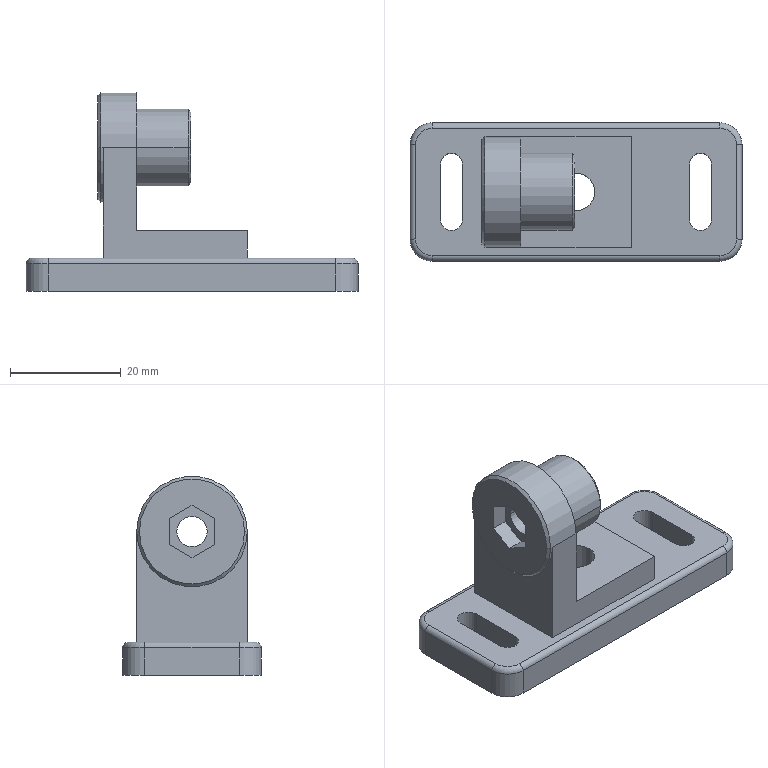Part | SolidWorks | features ICE 6, Chamfer 3, Extrusion 1, Fillet 1 | 1 solid | 55 faces | box 60 x 25 x 36 mm | volume 14469 mm3 | plane 25 | cylinder 20 | cone 6 | torus 4 | commonest cylinder face diameters 2 x4 4 x4 8 x4 5.5 x2 6.8 x2 13.9 x2
STEP:
#1=CARTESIAN_POINT('',(-0.2,6.45,26.));
#2=VERTEX_POINT('',#1);
#3=CARTESIAN_POINT('',(-0.2,-6.45,26.));
#4=VERTEX_POINT('',#3);
#5=CARTESIAN_POINT('',(-0.2,0.,26.));
#6=DIRECTION('',(1.,0.,0.));
#7=DIRECTION('',(0.,1.,0.));
#8=AXIS2_PLACEMENT_3D('',#5,#6,#7);
#9=CIRCLE('',#8,6.45);
#10=EDGE_CURVE('',#2,#4,#9,.T.);
#11=ORIENTED_EDGE('',*,*,#10,.F.);
#12=CARTESIAN_POINT('',(-0.7,6.95,26.));
#13=VERTEX_POINT('',#12);
#14=CARTESIAN_POINT('',(-0.2,6.45,26.));
#15=DIRECTION('',(-0.7071,0.7071,0.));
#16=VECTOR('',#15,1000.);
#17=LINE('',#14,#16);
#18=EDGE_CURVE('',#2,#13,#17,.T.);
#19=ORIENTED_EDGE('',*,*,#18,.T.);
#20=CARTESIAN_POINT('',(-0.7,-6.95,26.));
#21=VERTEX_POINT('',#20);
#22=CARTESIAN_POINT('',(-0.7,0.,26.));
#23=DIRECTION('',(-1.,0.,0.));
#24=DIRECTION('',(0.,1.,0.));
#25=AXIS2_PLACEMENT_3D('',#22,#23,#24);
#26=CIRCLE('',#25,6.95);
#27=EDGE_CURVE('',#21,#13,#26,.T.);
#28=ORIENTED_EDGE('',*,*,#27,.F.);
#29=CARTESIAN_POINT('',(-0.2,-6.45,26.));
#30=DIRECTION('',(-0.7071,-0.7071,0.));
#31=VECTOR('',#30,1000.);
#32=LINE('',#29,#31);
#33=EDGE_CURVE('',#4,#21,#32,.T.);
#34=ORIENTED_EDGE('',*,*,#33,.F.);
#35=EDGE_LOOP('',(#11,#19,#28,#34));
#36=FACE_OUTER_BOUND('',#35,.T.);
#37=CARTESIAN_POINT('',(-0.2,0.,26.));
#38=DIRECTION('',(-1.,0.,0.));
#39=DIRECTION('',(0.,-1.,0.));
#40=AXIS2_PLACEMENT_3D('',#37,#38,#39);
#41=CONICAL_SURFACE('',#40,6.45,0.7854);
#42=ADVANCED_FACE('',(#36),#41,.T.);
#43=ORIENTED_EDGE('',*,*,#27,.T.);
#44=CARTESIAN_POINT('',(-10.,6.95,26.));
#45=VERTEX_POINT('',#44);
#46=CARTESIAN_POINT('',(-0.2,6.95,26.));
#47=DIRECTION('',(-1.,0.,0.));
#48=VECTOR('',#47,1000.);
#49=LINE('',#46,#48);
#50=EDGE_CURVE('',#13,#45,#49,.T.);
#51=ORIENTED_EDGE('',*,*,#50,.T.);
#52=CARTESIAN_POINT('',(-10.,-6.95,26.));
#53=VERTEX_POINT('',#52);
#54=CARTESIAN_POINT('',(-10.,0.,26.));
#55=DIRECTION('',(1.,0.,0.));
#56=DIRECTION('',(0.,-1.,0.));
#57=AXIS2_PLACEMENT_3D('',#54,#55,#56);
#58=CIRCLE('',#57,6.95);
#59=EDGE_CURVE('',#45,#53,#58,.T.);
#60=ORIENTED_EDGE('',*,*,#59,.T.);
#61=CARTESIAN_POINT('',(-0.2,-6.95,26.));
#62=DIRECTION('',(-1.,0.,0.));
#63=VECTOR('',#62,1000.);
#64=LINE('',#61,#63);
#65=EDGE_CURVE('',#21,#53,#64,.T.);
#66=ORIENTED_EDGE('',*,*,#65,.F.);
#67=EDGE_LOOP('',(#43,#51,#60,#66));
#68=FACE_OUTER_BOUND('',#67,.T.);
#69=CARTESIAN_POINT('',(-0.2,0.,26.));
#70=DIRECTION('',(-1.,0.,0.));
#71=DIRECTION('',(0.,-1.,0.));
#72=AXIS2_PLACEMENT_3D('',#69,#70,#71);
#73=CYLINDRICAL_SURFACE('',#72,6.95);
#74=ADVANCED_FACE('',(#68),#73,.T.);
#75=CARTESIAN_POINT('',(-17.,-9.5,26.));
#76=VERTEX_POINT('',#75);
#77=CARTESIAN_POINT('',(-17.,9.5,26.));
#78=VERTEX_POINT('',#77);
#79=CARTESIAN_POINT('',(-17.,0.,26.));
#80=DIRECTION('',(-1.,0.,0.));
#81=DIRECTION('',(0.,-1.,0.));
#82=AXIS2_PLACEMENT_3D('',#79,#80,#81);
#83=CIRCLE('',#82,9.5);
#84=EDGE_CURVE('',#76,#78,#83,.T.);
#85=ORIENTED_EDGE('',*,*,#84,.F.);
#86=CARTESIAN_POINT('',(-16.5,-10.,26.));
#87=VERTEX_POINT('',#86);
#88=CARTESIAN_POINT('',(-17.,-9.5,26.));
#89=DIRECTION('',(0.7071,-0.7071,0.));
#90=VECTOR('',#89,1000.);
#91=LINE('',#88,#90);
#92=EDGE_CURVE('',#76,#87,#91,.T.);
#93=ORIENTED_EDGE('',*,*,#92,.T.);
#94=CARTESIAN_POINT('',(-16.5,10.,26.));
#95=VERTEX_POINT('',#94);
#96=CARTESIAN_POINT('',(-16.5,0.,26.));
#97=DIRECTION('',(1.,0.,0.));
#98=DIRECTION('',(0.,-1.,0.));
#99=AXIS2_PLACEMENT_3D('',#96,#97,#98);
#100=CIRCLE('',#99,10.);
#101=EDGE_CURVE('',#95,#87,#100,.T.);
#102=ORIENTED_EDGE('',*,*,#101,.F.);
#103=CARTESIAN_POINT('',(-17.,9.5,26.));
#104=DIRECTION('',(0.7071,0.7071,0.));
#105=VECTOR('',#104,1000.);
#106=LINE('',#103,#105);
#107=EDGE_CURVE('',#78,#95,#106,.T.);
#108=ORIENTED_EDGE('',*,*,#107,.F.);
#109=EDGE_LOOP('',(#85,#93,#102,#108));
#110=FACE_OUTER_BOUND('',#109,.T.);
#111=CARTESIAN_POINT('',(-17.,0.,26.));
#112=DIRECTION('',(1.,0.,0.));
#113=DIRECTION('',(0.,1.,0.));
#114=AXIS2_PLACEMENT_3D('',#111,#112,#113);
#115=CONICAL_SURFACE('',#114,9.5,0.7854);
#116=ADVANCED_FACE('',(#110),#115,.T.);
#117=CARTESIAN_POINT('',(-10.,10.,26.));
#118=VERTEX_POINT('',#117);
#119=CARTESIAN_POINT('',(-16.,10.,26.));
#120=VERTEX_POINT('',#119);
#121=CARTESIAN_POINT('',(30.,10.,26.));
#122=DIRECTION('',(-1.,0.,0.));
#123=VECTOR('',#122,1000.);
#124=LINE('',#121,#123);
#125=EDGE_CURVE('',#118,#120,#124,.T.);
#126=ORIENTED_EDGE('',*,*,#125,.T.);
#127=CARTESIAN_POINT('',(30.,10.,26.));
#128=DIRECTION('',(-1.,0.,0.));
#129=VECTOR('',#128,1000.);
#130=LINE('',#127,#129);
#131=EDGE_CURVE('',#120,#95,#130,.T.);
#132=ORIENTED_EDGE('',*,*,#131,.T.);
#133=ORIENTED_EDGE('',*,*,#101,.T.);
#134=CARTESIAN_POINT('',(-16.,-10.,26.));
#135=VERTEX_POINT('',#134);
#136=CARTESIAN_POINT('',(30.,-10.,26.));
#137=DIRECTION('',(-1.,0.,0.));
#138=VECTOR('',#137,1000.);
#139=LINE('',#136,#138);
#140=EDGE_CURVE('',#135,#87,#139,.T.);
#141=ORIENTED_EDGE('',*,*,#140,.F.);
#142=CARTESIAN_POINT('',(-10.,-10.,26.));
#143=VERTEX_POINT('',#142);
#144=CARTESIAN_POINT('',(30.,-10.,26.));
#145=DIRECTION('',(-1.,0.,0.));
#146=VECTOR('',#145,1000.);
#147=LINE('',#144,#146);
#148=EDGE_CURVE('',#143,#135,#147,.T.);
#149=ORIENTED_EDGE('',*,*,#148,.F.);
#150=CARTESIAN_POINT('',(-10.,0.,26.));
#151=DIRECTION('',(1.,0.,0.));
#152=DIRECTION('',(0.,-1.,0.));
#153=AXIS2_PLACEMENT_3D('',#150,#151,#152);
#154=CIRCLE('',#153,10.);
#155=EDGE_CURVE('',#118,#143,#154,.T.);
#156=ORIENTED_EDGE('',*,*,#155,.F.);
#157=EDGE_LOOP('',(#126,#132,#133,#141,#149,#156));
#158=FACE_OUTER_BOUND('',#157,.T.);
#159=CARTESIAN_POINT('',(30.,0.,26.));
#160=DIRECTION('',(-1.,0.,0.));
#161=DIRECTION('',(0.,-1.,0.));
#162=AXIS2_PLACEMENT_3D('',#159,#160,#161);
#163=CYLINDRICAL_SURFACE('',#162,10.);
#164=ADVANCED_FACE('',(#158),#163,.T.);
#165=CARTESIAN_POINT('',(3.4,0.,1.));
#166=VERTEX_POINT('',#165);
#167=CARTESIAN_POINT('',(-3.4,0.,1.));
#168=VERTEX_POINT('',#167);
#169=CARTESIAN_POINT('',(0.,0.,1.));
#170=DIRECTION('',(0.,0.,-1.));
#171=DIRECTION('',(1.,0.,0.));
#172=AXIS2_PLACEMENT_3D('',#169,#170,#171);
#173=CIRCLE('',#172,3.4);
#174=EDGE_CURVE('',#166,#168,#173,.T.);
#175=ORIENTED_EDGE('',*,*,#174,.F.);
#176=CARTESIAN_POINT('',(4.4,0.,0.));
#177=VERTEX_POINT('',#176);
#178=CARTESIAN_POINT('',(4.4,0.,0.));
#179=DIRECTION('',(0.7071,0.,-0.7071));
#180=VECTOR('',#179,1000.);
#181=LINE('',#178,#180);
#182=EDGE_CURVE('',#166,#177,#181,.T.);
#183=ORIENTED_EDGE('',*,*,#182,.T.);
#184=CARTESIAN_POINT('',(-4.4,0.,0.));
#185=VERTEX_POINT('',#184);
#186=CARTESIAN_POINT('',(0.,0.,0.));
#187=DIRECTION('',(0.,0.,1.));
#188=DIRECTION('',(1.,0.,0.));
#189=AXIS2_PLACEMENT_3D('',#186,#187,#188);
#190=CIRCLE('',#189,4.4);
#191=EDGE_CURVE('',#185,#177,#190,.T.);
#192=ORIENTED_EDGE('',*,*,#191,.F.);
#193=CARTESIAN_POINT('',(-4.4,0.,0.));
#194=DIRECTION('',(-0.7071,0.,-0.7071));
#195=VECTOR('',#194,1000.);
#196=LINE('',#193,#195);
#197=EDGE_CURVE('',#168,#185,#196,.T.);
#198=ORIENTED_EDGE('',*,*,#197,.F.);
#199=EDGE_LOOP('',(#175,#183,#192,#198));
#200=FACE_OUTER_BOUND('',#199,.T.);
#201=CARTESIAN_POINT('',(0.,0.,0.));
#202=DIRECTION('',(0.,0.,-1.));
#203=DIRECTION('',(-1.,0.,0.));
#204=AXIS2_PLACEMENT_3D('',#201,#202,#203);
#205=CONICAL_SURFACE('',#204,4.4,0.7854);
#206=ADVANCED_FACE('',(#200),#205,.F.);
#207=CARTESIAN_POINT('',(-3.4,0.,11.));
#208=VERTEX_POINT('',#207);
#209=CARTESIAN_POINT('',(3.4,0.,11.));
#210=VERTEX_POINT('',#209);
#211=CARTESIAN_POINT('',(0.,0.,11.));
#212=DIRECTION('',(0.,0.,1.));
#213=DIRECTION('',(1.,0.,0.));
#214=AXIS2_PLACEMENT_3D('',#211,#212,#213);
#215=CIRCLE('',#214,3.4);
#216=EDGE_CURVE('',#208,#210,#215,.T.);
#217=ORIENTED_EDGE('',*,*,#216,.T.);
#218=CARTESIAN_POINT('',(3.4,0.,6.));
#219=DIRECTION('',(0.,0.,-1.));
#220=VECTOR('',#219,1000.);
#221=LINE('',#218,#220);
#222=EDGE_CURVE('',#210,#166,#221,.T.);
#223=ORIENTED_EDGE('',*,*,#222,.T.);
#224=ORIENTED_EDGE('',*,*,#174,.T.);
#225=CARTESIAN_POINT('',(-3.4,0.,6.));
#226=DIRECTION('',(0.,0.,-1.));
#227=VECTOR('',#226,1000.);
#228=LINE('',#225,#227);
#229=EDGE_CURVE('',#208,#168,#228,.T.);
#230=ORIENTED_EDGE('',*,*,#229,.F.);
#231=EDGE_LOOP('',(#217,#223,#224,#230));
#232=FACE_OUTER_BOUND('',#231,.T.);
#233=CARTESIAN_POINT('',(0.,0.,6.));
#234=DIRECTION('',(0.,0.,-1.));
#235=DIRECTION('',(-1.,0.,0.));
#236=AXIS2_PLACEMENT_3D('',#233,#234,#235);
#237=CYLINDRICAL_SURFACE('',#236,3.4);
#238=ADVANCED_FACE('',(#232),#237,.F.);
#239=CARTESIAN_POINT('',(-0.2,-2.75,26.));
#240=VERTEX_POINT('',#239);
#241=CARTESIAN_POINT('',(-0.2,2.75,26.));
#242=VERTEX_POINT('',#241);
#243=CARTESIAN_POINT('',(-0.2,0.,26.));
#244=DIRECTION('',(1.,0.,0.));
#245=DIRECTION('',(0.,1.,0.));
#246=AXIS2_PLACEMENT_3D('',#243,#244,#245);
#247=CIRCLE('',#246,2.75);
#248=EDGE_CURVE('',#240,#242,#247,.T.);
#249=ORIENTED_EDGE('',*,*,#248,.T.);
#250=CARTESIAN_POINT('',(-14.,2.75,26.));
#251=VERTEX_POINT('',#250);
#252=CARTESIAN_POINT('',(30.,2.75,26.));
#253=DIRECTION('',(-1.,0.,0.));
#254=VECTOR('',#253,1000.);
#255=LINE('',#252,#254);
#256=EDGE_CURVE('',#242,#251,#255,.T.);
#257=ORIENTED_EDGE('',*,*,#256,.T.);
#258=CARTESIAN_POINT('',(-14.,-2.75,26.));
#259=VERTEX_POINT('',#258);
#260=CARTESIAN_POINT('',(-14.,0.,26.));
#261=DIRECTION('',(1.,0.,0.));
#262=DIRECTION('',(0.,0.,1.));
#263=AXIS2_PLACEMENT_3D('',#260,#261,#262);
#264=CIRCLE('',#263,2.75);
#265=EDGE_CURVE('',#259,#251,#264,.T.);
#266=ORIENTED_EDGE('',*,*,#265,.F.);
#267=CARTESIAN_POINT('',(30.,-2.75,26.));
#268=DIRECTION('',(-1.,0.,0.));
#269=VECTOR('',#268,1000.);
#270=LINE('',#267,#269);
#271=EDGE_CURVE('',#240,#259,#270,.T.);
#272=ORIENTED_EDGE('',*,*,#271,.F.);
#273=EDGE_LOOP('',(#249,#257,#266,#272));
#274=FACE_OUTER_BOUND('',#273,.T.);
#275=CARTESIAN_POINT('',(30.,0.,26.));
#276=DIRECTION('',(-1.,0.,0.));
#277=DIRECTION('',(0.,-1.,0.));
#278=AXIS2_PLACEMENT_3D('',#275,#276,#277);
#279=CYLINDRICAL_SURFACE('',#278,2.75);
#280=ADVANCED_FACE('',(#274),#279,.F.);
#281=CARTESIAN_POINT('',(-10.,-10.,11.));
#282=VERTEX_POINT('',#281);
#283=CARTESIAN_POINT('',(-10.,-10.,36.));
#284=DIRECTION('',(0.,0.,-1.));
#285=VECTOR('',#284,1000.);
#286=LINE('',#283,#285);
#287=EDGE_CURVE('',#143,#282,#286,.T.);
#288=ORIENTED_EDGE('',*,*,#287,.T.);
#289=CARTESIAN_POINT('',(-10.,10.,11.));
#290=VERTEX_POINT('',#289);
#291=CARTESIAN_POINT('',(-10.,-10.,11.));
#292=DIRECTION('',(0.,-1.,0.));
#293=VECTOR('',#292,1000.);
#294=LINE('',#291,#293);
#295=EDGE_CURVE('',#290,#282,#294,.T.);
#296=ORIENTED_EDGE('',*,*,#295,.F.);
#297=CARTESIAN_POINT('',(-10.,10.,36.));
#298=DIRECTION('',(0.,0.,-1.));
#299=VECTOR('',#298,1000.);
#300=LINE('',#297,#299);
#301=EDGE_CURVE('',#118,#290,#300,.T.);
#302=ORIENTED_EDGE('',*,*,#301,.F.);
#303=ORIENTED_EDGE('',*,*,#155,.T.);
#304=EDGE_LOOP('',(#288,#296,#302,#303));
#305=FACE_OUTER_BOUND('',#304,.T.);
#306=CARTESIAN_POINT('',(-10.,0.,26.));
#307=DIRECTION('',(1.,0.,0.));
#308=DIRECTION('',(0.,-1.,0.));
#309=AXIS2_PLACEMENT_3D('',#306,#307,#308);
#310=CIRCLE('',#309,6.95);
#311=EDGE_CURVE('',#53,#45,#310,.T.);
#312=ORIENTED_EDGE('',*,*,#311,.F.);
#313=ORIENTED_EDGE('',*,*,#59,.F.);
#314=EDGE_LOOP('',(#312,#313));
#315=FACE_BOUND('',#314,.T.);
#316=CARTESIAN_POINT('',(-10.,10.,36.));
#317=DIRECTION('',(-1.,0.,0.));
#318=DIRECTION('',(0.,-1.,0.));
#319=AXIS2_PLACEMENT_3D('',#316,#317,#318);
#320=PLANE('',#319);
#321=ADVANCED_FACE('',(#305,#315),#320,.F.);
#322=ORIENTED_EDGE('',*,*,#256,.F.);
#323=CARTESIAN_POINT('',(-0.2,0.,26.));
#324=DIRECTION('',(1.,0.,0.));
#325=DIRECTION('',(0.,1.,0.));
#326=AXIS2_PLACEMENT_3D('',#323,#324,#325);
#327=CIRCLE('',#326,2.75);
#328=EDGE_CURVE('',#242,#240,#327,.T.);
#329=ORIENTED_EDGE('',*,*,#328,.T.);
#330=ORIENTED_EDGE('',*,*,#271,.T.);
#331=CARTESIAN_POINT('',(-14.,0.,26.));
#332=DIRECTION('',(1.,0.,0.));
#333=DIRECTION('',(0.,0.,1.));
#334=AXIS2_PLACEMENT_3D('',#331,#332,#333);
#335=CIRCLE('',#334,2.75);
#336=EDGE_CURVE('',#251,#259,#335,.T.);
#337=ORIENTED_EDGE('',*,*,#336,.F.);
#338=EDGE_LOOP('',(#322,#329,#330,#337));
#339=FACE_OUTER_BOUND('',#338,.T.);
#340=CARTESIAN_POINT('',(30.,0.,26.));
#341=DIRECTION('',(-1.,0.,0.));
#342=DIRECTION('',(0.,-1.,0.));
#343=AXIS2_PLACEMENT_3D('',#340,#341,#342);
#344=CYLINDRICAL_SURFACE('',#343,2.75);
#345=ADVANCED_FACE('',(#339),#344,.F.);
#346=CARTESIAN_POINT('',(-17.,0.,26.));
#347=DIRECTION('',(-1.,0.,0.));
#348=DIRECTION('',(0.,-1.,0.));
#349=AXIS2_PLACEMENT_3D('',#346,#347,#348);
#350=CIRCLE('',#349,9.5);
#351=EDGE_CURVE('',#78,#76,#350,.T.);
#352=ORIENTED_EDGE('',*,*,#351,.T.);
#353=ORIENTED_EDGE('',*,*,#84,.T.);
#354=EDGE_LOOP('',(#352,#353));
#355=FACE_OUTER_BOUND('',#354,.T.);
#356=CARTESIAN_POINT('',(-17.,4.102,23.635));
#357=VERTEX_POINT('',#356);
#358=CARTESIAN_POINT('',(-17.,4.098,28.37));
#359=VERTEX_POINT('',#358);
#360=CARTESIAN_POINT('',(-17.,4.1,26.003));
#361=DIRECTION('',(0.,-0.0006348,1.));
#362=VECTOR('',#361,1000.);
#363=LINE('',#360,#362);
#364=EDGE_CURVE('',#357,#359,#363,.T.);
#365=ORIENTED_EDGE('',*,*,#364,.T.);
#366=CARTESIAN_POINT('',(-17.,-0.003006,30.734));
#367=VERTEX_POINT('',#366);
#368=CARTESIAN_POINT('',(-17.,2.048,29.552));
#369=DIRECTION('',(0.,-0.8663,0.4995));
#370=VECTOR('',#369,1000.);
#371=LINE('',#368,#370);
#372=EDGE_CURVE('',#359,#367,#371,.T.);
#373=ORIENTED_EDGE('',*,*,#372,.T.);
#374=CARTESIAN_POINT('',(-17.,-4.102,28.365));
#375=VERTEX_POINT('',#374);
#376=CARTESIAN_POINT('',(-17.,-2.052,29.549));
#377=DIRECTION('',(0.,-0.8657,-0.5005));
#378=VECTOR('',#377,1000.);
#379=LINE('',#376,#378);
#380=EDGE_CURVE('',#367,#375,#379,.T.);
#381=ORIENTED_EDGE('',*,*,#380,.T.);
#382=CARTESIAN_POINT('',(-17.,-4.098,23.63));
#383=VERTEX_POINT('',#382);
#384=CARTESIAN_POINT('',(-17.,-4.1,25.997));
#385=DIRECTION('',(0.,0.0006348,-1.));
#386=VECTOR('',#385,1000.);
#387=LINE('',#384,#386);
#388=EDGE_CURVE('',#375,#383,#387,.T.);
#389=ORIENTED_EDGE('',*,*,#388,.T.);
#390=CARTESIAN_POINT('',(-17.,0.003006,21.266));
#391=VERTEX_POINT('',#390);
#392=CARTESIAN_POINT('',(-17.,-2.048,22.448));
#393=DIRECTION('',(0.,0.8663,-0.4995));
#394=VECTOR('',#393,1000.);
#395=LINE('',#392,#394);
#396=EDGE_CURVE('',#383,#391,#395,.T.);
#397=ORIENTED_EDGE('',*,*,#396,.T.);
#398=CARTESIAN_POINT('',(-17.,2.052,22.451));
#399=DIRECTION('',(0.,0.8657,0.5005));
#400=VECTOR('',#399,1000.);
#401=LINE('',#398,#400);
#402=EDGE_CURVE('',#391,#357,#401,.T.);
#403=ORIENTED_EDGE('',*,*,#402,.T.);
#404=EDGE_LOOP('',(#365,#373,#381,#389,#397,#403));
#405=FACE_BOUND('',#404,.T.);
#406=CARTESIAN_POINT('',(-17.,0.,26.));
#407=DIRECTION('',(-1.,0.,0.));
#408=DIRECTION('',(0.,-1.,0.));
#409=AXIS2_PLACEMENT_3D('',#406,#407,#408);
#410=PLANE('',#409);
#411=ADVANCED_FACE('',(#355,#405),#410,.T.);
#412=CARTESIAN_POINT('',(20.5,5.,6.));
#413=VERTEX_POINT('',#412);
#414=CARTESIAN_POINT('',(20.5,-5.,6.));
#415=VERTEX_POINT('',#414);
#416=CARTESIAN_POINT('',(20.5,5.,6.));
#417=DIRECTION('',(0.,-1.,0.));
#418=VECTOR('',#417,1000.);
#419=LINE('',#416,#418);
#420=EDGE_CURVE('',#413,#415,#419,.T.);
#421=ORIENTED_EDGE('',*,*,#420,.F.);
#422=CARTESIAN_POINT('',(24.5,5.,6.));
#423=VERTEX_POINT('',#422);
#424=CARTESIAN_POINT('',(22.5,5.,6.));
#425=DIRECTION('',(0.,0.,1.));
#426=DIRECTION('',(-1.,0.,0.));
#427=AXIS2_PLACEMENT_3D('',#424,#425,#426);
#428=CIRCLE('',#427,2.);
#429=EDGE_CURVE('',#423,#413,#428,.T.);
#430=ORIENTED_EDGE('',*,*,#429,.F.);
#431=CARTESIAN_POINT('',(24.5,-5.,6.));
#432=VERTEX_POINT('',#431);
#433=CARTESIAN_POINT('',(24.5,5.,6.));
#434=DIRECTION('',(0.,1.,0.));
#435=VECTOR('',#434,1000.);
#436=LINE('',#433,#435);
#437=EDGE_CURVE('',#432,#423,#436,.T.);
#438=ORIENTED_EDGE('',*,*,#437,.F.);
#439=CARTESIAN_POINT('',(22.5,-5.,6.));
#440=DIRECTION('',(0.,0.,1.));
#441=DIRECTION('',(-1.,0.,0.));
#442=AXIS2_PLACEMENT_3D('',#439,#440,#441);
#443=CIRCLE('',#442,2.);
#444=EDGE_CURVE('',#415,#432,#443,.T.);
#445=ORIENTED_EDGE('',*,*,#444,.F.);
#446=EDGE_LOOP('',(#421,#430,#438,#445));
#447=FACE_BOUND('',#446,.T.);
#448=CARTESIAN_POINT('',(-24.5,5.,6.));
#449=VERTEX_POINT('',#448);
#450=CARTESIAN_POINT('',(-24.5,-5.,6.));
#451=VERTEX_POINT('',#450);
#452=CARTESIAN_POINT('',(-24.5,5.,6.));
#453=DIRECTION('',(0.,-1.,0.));
#454=VECTOR('',#453,1000.);
#455=LINE('',#452,#454);
#456=EDGE_CURVE('',#449,#451,#455,.T.);
#457=ORIENTED_EDGE('',*,*,#456,.F.);
#458=CARTESIAN_POINT('',(-20.5,5.,6.));
#459=VERTEX_POINT('',#458);
#460=CARTESIAN_POINT('',(-22.5,5.,6.));
#461=DIRECTION('',(0.,0.,1.));
#462=DIRECTION('',(1.,0.,0.));
#463=AXIS2_PLACEMENT_3D('',#460,#461,#462);
#464=CIRCLE('',#463,2.);
#465=EDGE_CURVE('',#459,#449,#464,.T.);
#466=ORIENTED_EDGE('',*,*,#465,.F.);
#467=CARTESIAN_POINT('',(-20.5,-5.,6.));
#468=VERTEX_POINT('',#467);
#469=CARTESIAN_POINT('',(-20.5,5.,6.));
#470=DIRECTION('',(0.,1.,0.));
#471=VECTOR('',#470,1000.);
#472=LINE('',#469,#471);
#473=EDGE_CURVE('',#468,#459,#472,.T.);
#474=ORIENTED_EDGE('',*,*,#473,.F.);
#475=CARTESIAN_POINT('',(-22.5,-5.,6.));
#476=DIRECTION('',(0.,0.,1.));
#477=DIRECTION('',(1.,0.,0.));
#478=AXIS2_PLACEMENT_3D('',#475,#476,#477);
#479=CIRCLE('',#478,2.);
#480=EDGE_CURVE('',#451,#468,#479,.T.);
#481=ORIENTED_EDGE('',*,*,#480,.F.);
#482=EDGE_LOOP('',(#457,#466,#474,#481));
#483=FACE_BOUND('',#482,.T.);
#484=CARTESIAN_POINT('',(26.,11.5,6.));
#485=VERTEX_POINT('',#484);
#486=CARTESIAN_POINT('',(-26.,11.5,6.));
#487=VERTEX_POINT('',#486);
#488=CARTESIAN_POINT('',(-26.,11.5,6.));
#489=DIRECTION('',(-1.,0.,0.));
#490=VECTOR('',#489,1000.);
#491=LINE('',#488,#490);
#492=EDGE_CURVE('',#485,#487,#491,.T.);
#493=ORIENTED_EDGE('',*,*,#492,.T.);
#494=CARTESIAN_POINT('',(-29.,8.5,6.));
#495=VERTEX_POINT('',#494);
#496=CARTESIAN_POINT('',(-26.,8.5,6.));
#497=DIRECTION('',(0.,0.,1.));
#498=DIRECTION('',(1.,0.,0.));
#499=AXIS2_PLACEMENT_3D('',#496,#497,#498);
#500=CIRCLE('',#499,3.);
#501=EDGE_CURVE('',#487,#495,#500,.T.);
#502=ORIENTED_EDGE('',*,*,#501,.T.);
#503=CARTESIAN_POINT('',(-29.,-8.5,6.));
#504=VERTEX_POINT('',#503);
#505=CARTESIAN_POINT('',(-29.,-8.5,6.));
#506=DIRECTION('',(0.,-1.,0.));
#507=VECTOR('',#506,1000.);
#508=LINE('',#505,#507);
#509=EDGE_CURVE('',#495,#504,#508,.T.);
#510=ORIENTED_EDGE('',*,*,#509,.T.);
#511=CARTESIAN_POINT('',(-26.,-11.5,6.));
#512=VERTEX_POINT('',#511);
#513=CARTESIAN_POINT('',(-26.,-8.5,6.));
#514=DIRECTION('',(0.,0.,1.));
#515=DIRECTION('',(1.,0.,0.));
#516=AXIS2_PLACEMENT_3D('',#513,#514,#515);
#517=CIRCLE('',#516,3.);
#518=EDGE_CURVE('',#504,#512,#517,.T.);
#519=ORIENTED_EDGE('',*,*,#518,.T.);
#520=CARTESIAN_POINT('',(26.,-11.5,6.));
#521=VERTEX_POINT('',#520);
#522=CARTESIAN_POINT('',(26.,-11.5,6.));
#523=DIRECTION('',(1.,0.,0.));
#524=VECTOR('',#523,1000.);
#525=LINE('',#522,#524);
#526=EDGE_CURVE('',#512,#521,#525,.T.);
#527=ORIENTED_EDGE('',*,*,#526,.T.);
#528=CARTESIAN_POINT('',(29.,-8.5,6.));
#529=VERTEX_POINT('',#528);
#530=CARTESIAN_POINT('',(26.,-8.5,6.));
#531=DIRECTION('',(0.,0.,1.));
#532=DIRECTION('',(1.,0.,0.));
#533=AXIS2_PLACEMENT_3D('',#530,#531,#532);
#534=CIRCLE('',#533,3.);
#535=EDGE_CURVE('',#521,#529,#534,.T.);
#536=ORIENTED_EDGE('',*,*,#535,.T.);
#537=CARTESIAN_POINT('',(29.,8.5,6.));
#538=VERTEX_POINT('',#537);
#539=CARTESIAN_POINT('',(29.,8.5,6.));
#540=DIRECTION('',(0.,1.,0.));
#541=VECTOR('',#540,1000.);
#542=LINE('',#539,#541);
#543=EDGE_CURVE('',#529,#538,#542,.T.);
#544=ORIENTED_EDGE('',*,*,#543,.T.);
#545=CARTESIAN_POINT('',(26.,8.5,6.));
#546=DIRECTION('',(0.,0.,1.));
#547=DIRECTION('',(1.,0.,0.));
#548=AXIS2_PLACEMENT_3D('',#545,#546,#547);
#549=CIRCLE('',#548,3.);
#550=EDGE_CURVE('',#538,#485,#549,.T.);
#551=ORIENTED_EDGE('',*,*,#550,.T.);
#552=EDGE_LOOP('',(#493,#502,#510,#519,#527,#536,#544,#551));
#553=FACE_OUTER_BOUND('',#552,.T.);
#554=CARTESIAN_POINT('',(10.,-10.,6.));
#555=VERTEX_POINT('',#554);
#556=CARTESIAN_POINT('',(10.,10.,6.));
#557=VERTEX_POINT('',#556);
#558=CARTESIAN_POINT('',(10.,-10.,6.));
#559=DIRECTION('',(0.,1.,0.));
#560=VECTOR('',#559,1000.);
#561=LINE('',#558,#560);
#562=EDGE_CURVE('',#555,#557,#561,.T.);
#563=ORIENTED_EDGE('',*,*,#562,.F.);
#564=CARTESIAN_POINT('',(-16.,-10.,6.));
#565=VERTEX_POINT('',#564);
#566=CARTESIAN_POINT('',(-16.,-10.,6.));
#567=DIRECTION('',(1.,0.,0.));
#568=VECTOR('',#567,1000.);
#569=LINE('',#566,#568);
#570=EDGE_CURVE('',#565,#555,#569,.T.);
#571=ORIENTED_EDGE('',*,*,#570,.F.);
#572=CARTESIAN_POINT('',(-16.,10.,6.));
#573=VERTEX_POINT('',#572);
#574=CARTESIAN_POINT('',(-16.,10.,6.));
#575=DIRECTION('',(0.,-1.,0.));
#576=VECTOR('',#575,1000.);
#577=LINE('',#574,#576);
#578=EDGE_CURVE('',#573,#565,#577,.T.);
#579=ORIENTED_EDGE('',*,*,#578,.F.);
#580=CARTESIAN_POINT('',(-16.,10.,6.));
#581=DIRECTION('',(-1.,0.,0.));
#582=VECTOR('',#581,1000.);
#583=LINE('',#580,#582);
#584=EDGE_CURVE('',#557,#573,#583,.T.);
#585=ORIENTED_EDGE('',*,*,#584,.F.);
#586=EDGE_LOOP('',(#563,#571,#579,#585));
#587=FACE_BOUND('',#586,.T.);
#588=CARTESIAN_POINT('',(-26.,-8.5,6.));
#589=DIRECTION('',(0.,0.,1.));
#590=DIRECTION('',(1.,0.,0.));
#591=AXIS2_PLACEMENT_3D('',#588,#589,#590);
#592=PLANE('',#591);
#593=ADVANCED_FACE('',(#447,#483,#553,#587),#592,.T.);
#594=CARTESIAN_POINT('',(-16.,0.,26.));
#595=DIRECTION('',(-1.,0.,0.));
#596=DIRECTION('',(0.,1.,0.));
#597=AXIS2_PLACEMENT_3D('',#594,#595,#596);
#598=CIRCLE('',#597,10.);
#599=EDGE_CURVE('',#120,#135,#598,.T.);
#600=ORIENTED_EDGE('',*,*,#599,.F.);
#601=CARTESIAN_POINT('',(-16.,10.,36.));
#602=DIRECTION('',(0.,0.,-1.));
#603=VECTOR('',#602,1000.);
#604=LINE('',#601,#603);
#605=EDGE_CURVE('',#120,#573,#604,.T.);
#606=ORIENTED_EDGE('',*,*,#605,.T.);
#607=ORIENTED_EDGE('',*,*,#578,.T.);
#608=CARTESIAN_POINT('',(-16.,-10.,36.));
#609=DIRECTION('',(0.,0.,-1.));
#610=VECTOR('',#609,1000.);
#611=LINE('',#608,#610);
#612=EDGE_CURVE('',#135,#565,#611,.T.);
#613=ORIENTED_EDGE('',*,*,#612,.F.);
#614=EDGE_LOOP('',(#600,#606,#607,#613));
#615=FACE_OUTER_BOUND('',#614,.T.);
#616=CARTESIAN_POINT('',(-16.,10.,36.));
#617=DIRECTION('',(1.,0.,0.));
#618=DIRECTION('',(0.,1.,0.));
#619=AXIS2_PLACEMENT_3D('',#616,#617,#618);
#620=PLANE('',#619);
#621=ADVANCED_FACE('',(#615),#620,.F.);
#622=ORIENTED_EDGE('',*,*,#191,.T.);
#623=CARTESIAN_POINT('',(0.,0.,0.));
#624=DIRECTION('',(0.,0.,1.));
#625=DIRECTION('',(1.,0.,0.));
#626=AXIS2_PLACEMENT_3D('',#623,#624,#625);
#627=CIRCLE('',#626,4.4);
#628=EDGE_CURVE('',#177,#185,#627,.T.);
#629=ORIENTED_EDGE('',*,*,#628,.T.);
#630=EDGE_LOOP('',(#622,#629));
#631=FACE_BOUND('',#630,.T.);
#632=CARTESIAN_POINT('',(-20.5,5.,0.));
#633=VERTEX_POINT('',#632);
#634=CARTESIAN_POINT('',(-24.5,5.,0.));
#635=VERTEX_POINT('',#634);
#636=CARTESIAN_POINT('',(-22.5,5.,0.));
#637=DIRECTION('',(0.,0.,1.));
#638=DIRECTION('',(1.,0.,0.));
#639=AXIS2_PLACEMENT_3D('',#636,#637,#638);
#640=CIRCLE('',#639,2.);
#641=EDGE_CURVE('',#633,#635,#640,.T.);
#642=ORIENTED_EDGE('',*,*,#641,.T.);
#643=CARTESIAN_POINT('',(-24.5,-5.,0.));
#644=VERTEX_POINT('',#643);
#645=CARTESIAN_POINT('',(-24.5,5.,0.));
#646=DIRECTION('',(0.,-1.,0.));
#647=VECTOR('',#646,1000.);
#648=LINE('',#645,#647);
#649=EDGE_CURVE('',#635,#644,#648,.T.);
#650=ORIENTED_EDGE('',*,*,#649,.T.);
#651=CARTESIAN_POINT('',(-20.5,-5.,0.));
#652=VERTEX_POINT('',#651);
#653=CARTESIAN_POINT('',(-22.5,-5.,0.));
#654=DIRECTION('',(0.,0.,1.));
#655=DIRECTION('',(1.,0.,0.));
#656=AXIS2_PLACEMENT_3D('',#653,#654,#655);
#657=CIRCLE('',#656,2.);
#658=EDGE_CURVE('',#644,#652,#657,.T.);
#659=ORIENTED_EDGE('',*,*,#658,.T.);
#660=CARTESIAN_POINT('',(-20.5,5.,0.));
#661=DIRECTION('',(0.,1.,0.));
#662=VECTOR('',#661,1000.);
#663=LINE('',#660,#662);
#664=EDGE_CURVE('',#652,#633,#663,.T.);
#665=ORIENTED_EDGE('',*,*,#664,.T.);
#666=EDGE_LOOP('',(#642,#650,#659,#665));
#667=FACE_BOUND('',#666,.T.);
#668=CARTESIAN_POINT('',(-30.,-8.5,0.));
#669=VERTEX_POINT('',#668);
#670=CARTESIAN_POINT('',(-26.,-12.5,0.));
#671=VERTEX_POINT('',#670);
#672=CARTESIAN_POINT('',(-26.,-8.5,0.));
#673=DIRECTION('',(0.,0.,1.));
#674=DIRECTION('',(1.,0.,0.));
#675=AXIS2_PLACEMENT_3D('',#672,#673,#674);
#676=CIRCLE('',#675,4.);
#677=EDGE_CURVE('',#669,#671,#676,.T.);
#678=ORIENTED_EDGE('',*,*,#677,.F.);
#679=CARTESIAN_POINT('',(-30.,8.5,0.));
#680=VERTEX_POINT('',#679);
#681=CARTESIAN_POINT('',(-30.,8.5,0.));
#682=DIRECTION('',(0.,-1.,0.));
#683=VECTOR('',#682,1000.);
#684=LINE('',#681,#683);
#685=EDGE_CURVE('',#680,#669,#684,.T.);
#686=ORIENTED_EDGE('',*,*,#685,.F.);
#687=CARTESIAN_POINT('',(-26.,12.5,0.));
#688=VERTEX_POINT('',#687);
#689=CARTESIAN_POINT('',(-26.,8.5,0.));
#690=DIRECTION('',(0.,0.,1.));
#691=DIRECTION('',(1.,0.,0.));
#692=AXIS2_PLACEMENT_3D('',#689,#690,#691);
#693=CIRCLE('',#692,4.);
#694=EDGE_CURVE('',#688,#680,#693,.T.);
#695=ORIENTED_EDGE('',*,*,#694,.F.);
#696=CARTESIAN_POINT('',(26.,12.5,0.));
#697=VERTEX_POINT('',#696);
#698=CARTESIAN_POINT('',(-26.,12.5,0.));
#699=DIRECTION('',(-1.,0.,0.));
#700=VECTOR('',#699,1000.);
#701=LINE('',#698,#700);
#702=EDGE_CURVE('',#697,#688,#701,.T.);
#703=ORIENTED_EDGE('',*,*,#702,.F.);
#704=CARTESIAN_POINT('',(30.,8.5,0.));
#705=VERTEX_POINT('',#704);
#706=CARTESIAN_POINT('',(26.,8.5,0.));
#707=DIRECTION('',(0.,0.,1.));
#708=DIRECTION('',(-1.,0.,0.));
#709=AXIS2_PLACEMENT_3D('',#706,#707,#708);
#710=CIRCLE('',#709,4.);
#711=EDGE_CURVE('',#705,#697,#710,.T.);
#712=ORIENTED_EDGE('',*,*,#711,.F.);
#713=CARTESIAN_POINT('',(30.,-8.5,0.));
#714=VERTEX_POINT('',#713);
#715=CARTESIAN_POINT('',(30.,8.5,0.));
#716=DIRECTION('',(0.,1.,0.));
#717=VECTOR('',#716,1000.);
#718=LINE('',#715,#717);
#719=EDGE_CURVE('',#714,#705,#718,.T.);
#720=ORIENTED_EDGE('',*,*,#719,.F.);
#721=CARTESIAN_POINT('',(26.,-12.5,0.));
#722=VERTEX_POINT('',#721);
#723=CARTESIAN_POINT('',(26.,-8.5,0.));
#724=DIRECTION('',(0.,0.,1.));
#725=DIRECTION('',(1.,0.,0.));
#726=AXIS2_PLACEMENT_3D('',#723,#724,#725);
#727=CIRCLE('',#726,4.);
#728=EDGE_CURVE('',#722,#714,#727,.T.);
#729=ORIENTED_EDGE('',*,*,#728,.F.);
#730=CARTESIAN_POINT('',(-26.,-12.5,0.));
#731=DIRECTION('',(1.,0.,0.));
#732=VECTOR('',#731,1000.);
#733=LINE('',#730,#732);
#734=EDGE_CURVE('',#671,#722,#733,.T.);
#735=ORIENTED_EDGE('',*,*,#734,.F.);
#736=EDGE_LOOP('',(#678,#686,#695,#703,#712,#720,#729,#735));
#737=FACE_OUTER_BOUND('',#736,.T.);
#738=CARTESIAN_POINT('',(24.5,5.,0.));
#739=VERTEX_POINT('',#738);
#740=CARTESIAN_POINT('',(20.5,5.,0.));
#741=VERTEX_POINT('',#740);
#742=CARTESIAN_POINT('',(22.5,5.,0.));
#743=DIRECTION('',(0.,0.,1.));
#744=DIRECTION('',(-1.,0.,0.));
#745=AXIS2_PLACEMENT_3D('',#742,#743,#744);
#746=CIRCLE('',#745,2.);
#747=EDGE_CURVE('',#739,#741,#746,.T.);
#748=ORIENTED_EDGE('',*,*,#747,.T.);
#749=CARTESIAN_POINT('',(20.5,-5.,0.));
#750=VERTEX_POINT('',#749);
#751=CARTESIAN_POINT('',(20.5,5.,0.));
#752=DIRECTION('',(0.,-1.,0.));
#753=VECTOR('',#752,1000.);
#754=LINE('',#751,#753);
#755=EDGE_CURVE('',#741,#750,#754,.T.);
#756=ORIENTED_EDGE('',*,*,#755,.T.);
#757=CARTESIAN_POINT('',(24.5,-5.,0.));
#758=VERTEX_POINT('',#757);
#759=CARTESIAN_POINT('',(22.5,-5.,0.));
#760=DIRECTION('',(0.,0.,1.));
#761=DIRECTION('',(-1.,0.,0.));
#762=AXIS2_PLACEMENT_3D('',#759,#760,#761);
#763=CIRCLE('',#762,2.);
#764=EDGE_CURVE('',#750,#758,#763,.T.);
#765=ORIENTED_EDGE('',*,*,#764,.T.);
#766=CARTESIAN_POINT('',(24.5,5.,0.));
#767=DIRECTION('',(0.,1.,0.));
#768=VECTOR('',#767,1000.);
#769=LINE('',#766,#768);
#770=EDGE_CURVE('',#758,#739,#769,.T.);
#771=ORIENTED_EDGE('',*,*,#770,.T.);
#772=EDGE_LOOP('',(#748,#756,#765,#771));
#773=FACE_BOUND('',#772,.T.);
#774=CARTESIAN_POINT('',(-26.,-8.5,0.));
#775=DIRECTION('',(0.,0.,1.));
#776=DIRECTION('',(1.,0.,0.));
#777=AXIS2_PLACEMENT_3D('',#774,#775,#776);
#778=PLANE('',#777);
#779=ADVANCED_FACE('',(#631,#667,#737,#773),#778,.F.);
#780=CARTESIAN_POINT('',(-26.,-12.5,5.));
#781=VERTEX_POINT('',#780);
#782=CARTESIAN_POINT('',(-26.,-12.5,6.));
#783=DIRECTION('',(0.,0.,-1.));
#784=VECTOR('',#783,1000.);
#785=LINE('',#782,#784);
#786=EDGE_CURVE('',#781,#671,#785,.T.);
#787=ORIENTED_EDGE('',*,*,#786,.F.);
#788=CARTESIAN_POINT('',(-30.,-8.5,5.));
#789=VERTEX_POINT('',#788);
#790=CARTESIAN_POINT('',(-26.,-8.5,5.));
#791=DIRECTION('',(0.,0.,-1.));
#792=DIRECTION('',(1.,0.,0.));
#793=AXIS2_PLACEMENT_3D('',#790,#791,#792);
#794=CIRCLE('',#793,4.);
#795=EDGE_CURVE('',#781,#789,#794,.T.);
#796=ORIENTED_EDGE('',*,*,#795,.T.);
#797=CARTESIAN_POINT('',(-30.,-8.5,6.));
#798=DIRECTION('',(0.,0.,-1.));
#799=VECTOR('',#798,1000.);
#800=LINE('',#797,#799);
#801=EDGE_CURVE('',#789,#669,#800,.T.);
#802=ORIENTED_EDGE('',*,*,#801,.T.);
#803=ORIENTED_EDGE('',*,*,#677,.T.);
#804=EDGE_LOOP('',(#787,#796,#802,#803));
#805=FACE_OUTER_BOUND('',#804,.T.);
#806=CARTESIAN_POINT('',(-26.,-8.5,6.));
#807=DIRECTION('',(0.,0.,-1.));
#808=DIRECTION('',(-1.,0.,0.));
#809=AXIS2_PLACEMENT_3D('',#806,#807,#808);
#810=CYLINDRICAL_SURFACE('',#809,4.);
#811=ADVANCED_FACE('',(#805),#810,.T.);
#812=CARTESIAN_POINT('',(26.,-12.5,5.));
#813=VERTEX_POINT('',#812);
#814=CARTESIAN_POINT('',(26.,-12.5,6.));
#815=DIRECTION('',(0.,0.,-1.));
#816=VECTOR('',#815,1000.);
#817=LINE('',#814,#816);
#818=EDGE_CURVE('',#813,#722,#817,.T.);
#819=ORIENTED_EDGE('',*,*,#818,.F.);
#820=CARTESIAN_POINT('',(-26.,-12.5,5.));
#821=DIRECTION('',(-1.,0.,0.));
#822=VECTOR('',#821,1000.);
#823=LINE('',#820,#822);
#824=EDGE_CURVE('',#813,#781,#823,.T.);
#825=ORIENTED_EDGE('',*,*,#824,.T.);
#826=ORIENTED_EDGE('',*,*,#786,.T.);
#827=ORIENTED_EDGE('',*,*,#734,.T.);
#828=EDGE_LOOP('',(#819,#825,#826,#827));
#829=FACE_OUTER_BOUND('',#828,.T.);
#830=CARTESIAN_POINT('',(-26.,-12.5,6.));
#831=DIRECTION('',(0.,1.,0.));
#832=DIRECTION('',(-1.,0.,0.));
#833=AXIS2_PLACEMENT_3D('',#830,#831,#832);
#834=PLANE('',#833);
#835=ADVANCED_FACE('',(#829),#834,.F.);
#836=CARTESIAN_POINT('',(30.,-8.5,5.));
#837=VERTEX_POINT('',#836);
#838=CARTESIAN_POINT('',(30.,-8.5,6.));
#839=DIRECTION('',(0.,0.,-1.));
#840=VECTOR('',#839,1000.);
#841=LINE('',#838,#840);
#842=EDGE_CURVE('',#837,#714,#841,.T.);
#843=ORIENTED_EDGE('',*,*,#842,.F.);
#844=CARTESIAN_POINT('',(26.,-8.5,5.));
#845=DIRECTION('',(0.,0.,-1.));
#846=DIRECTION('',(1.,0.,0.));
#847=AXIS2_PLACEMENT_3D('',#844,#845,#846);
#848=CIRCLE('',#847,4.);
#849=EDGE_CURVE('',#837,#813,#848,.T.);
#850=ORIENTED_EDGE('',*,*,#849,.T.);
#851=ORIENTED_EDGE('',*,*,#818,.T.);
#852=ORIENTED_EDGE('',*,*,#728,.T.);
#853=EDGE_LOOP('',(#843,#850,#851,#852));
#854=FACE_OUTER_BOUND('',#853,.T.);
#855=CARTESIAN_POINT('',(26.,-8.5,6.));
#856=DIRECTION('',(0.,0.,-1.));
#857=DIRECTION('',(-1.,0.,0.));
#858=AXIS2_PLACEMENT_3D('',#855,#856,#857);
#859=CYLINDRICAL_SURFACE('',#858,4.);
#860=ADVANCED_FACE('',(#854),#859,.T.);
#861=CARTESIAN_POINT('',(30.,8.5,5.));
#862=VERTEX_POINT('',#861);
#863=CARTESIAN_POINT('',(30.,8.5,6.));
#864=DIRECTION('',(0.,0.,-1.));
#865=VECTOR('',#864,1000.);
#866=LINE('',#863,#865);
#867=EDGE_CURVE('',#862,#705,#866,.T.);
#868=ORIENTED_EDGE('',*,*,#867,.F.);
#869=CARTESIAN_POINT('',(30.,-8.5,5.));
#870=DIRECTION('',(0.,-1.,0.));
#871=VECTOR('',#870,1000.);
#872=LINE('',#869,#871);
#873=EDGE_CURVE('',#862,#837,#872,.T.);
#874=ORIENTED_EDGE('',*,*,#873,.T.);
#875=ORIENTED_EDGE('',*,*,#842,.T.);
#876=ORIENTED_EDGE('',*,*,#719,.T.);
#877=EDGE_LOOP('',(#868,#874,#875,#876));
#878=FACE_OUTER_BOUND('',#877,.T.);
#879=CARTESIAN_POINT('',(30.,8.5,6.));
#880=DIRECTION('',(-1.,0.,0.));
#881=DIRECTION('',(0.,-1.,0.));
#882=AXIS2_PLACEMENT_3D('',#879,#880,#881);
#883=PLANE('',#882);
#884=ADVANCED_FACE('',(#878),#883,.F.);
#885=CARTESIAN_POINT('',(26.,12.5,5.));
#886=VERTEX_POINT('',#885);
#887=CARTESIAN_POINT('',(26.,12.5,6.));
#888=DIRECTION('',(0.,0.,-1.));
#889=VECTOR('',#888,1000.);
#890=LINE('',#887,#889);
#891=EDGE_CURVE('',#886,#697,#890,.T.);
#892=ORIENTED_EDGE('',*,*,#891,.F.);
#893=CARTESIAN_POINT('',(26.,8.5,5.));
#894=DIRECTION('',(0.,0.,-1.));
#895=DIRECTION('',(1.,0.,0.));
#896=AXIS2_PLACEMENT_3D('',#893,#894,#895);
#897=CIRCLE('',#896,4.);
#898=EDGE_CURVE('',#886,#862,#897,.T.);
#899=ORIENTED_EDGE('',*,*,#898,.T.);
#900=ORIENTED_EDGE('',*,*,#867,.T.);
#901=ORIENTED_EDGE('',*,*,#711,.T.);
#902=EDGE_LOOP('',(#892,#899,#900,#901));
#903=FACE_OUTER_BOUND('',#902,.T.);
#904=CARTESIAN_POINT('',(26.,8.5,6.));
#905=DIRECTION('',(0.,0.,-1.));
#906=DIRECTION('',(-1.,0.,0.));
#907=AXIS2_PLACEMENT_3D('',#904,#905,#906);
#908=CYLINDRICAL_SURFACE('',#907,4.);
#909=ADVANCED_FACE('',(#903),#908,.T.);
#910=CARTESIAN_POINT('',(-26.,12.5,5.));
#911=VERTEX_POINT('',#910);
#912=CARTESIAN_POINT('',(-26.,12.5,6.));
#913=DIRECTION('',(0.,0.,-1.));
#914=VECTOR('',#913,1000.);
#915=LINE('',#912,#914);
#916=EDGE_CURVE('',#911,#688,#915,.T.);
#917=ORIENTED_EDGE('',*,*,#916,.F.);
#918=CARTESIAN_POINT('',(26.,12.5,5.));
#919=DIRECTION('',(1.,0.,0.));
#920=VECTOR('',#919,1000.);
#921=LINE('',#918,#920);
#922=EDGE_CURVE('',#911,#886,#921,.T.);
#923=ORIENTED_EDGE('',*,*,#922,.T.);
#924=ORIENTED_EDGE('',*,*,#891,.T.);
#925=ORIENTED_EDGE('',*,*,#702,.T.);
#926=EDGE_LOOP('',(#917,#923,#924,#925));
#927=FACE_OUTER_BOUND('',#926,.T.);
#928=CARTESIAN_POINT('',(-26.,12.5,6.));
#929=DIRECTION('',(0.,-1.,0.));
#930=DIRECTION('',(0.,0.,-1.));
#931=AXIS2_PLACEMENT_3D('',#928,#929,#930);
#932=PLANE('',#931);
#933=ADVANCED_FACE('',(#927),#932,.F.);
#934=CARTESIAN_POINT('',(-30.,8.5,5.));
#935=VERTEX_POINT('',#934);
#936=CARTESIAN_POINT('',(-30.,8.5,6.));
#937=DIRECTION('',(0.,0.,-1.));
#938=VECTOR('',#937,1000.);
#939=LINE('',#936,#938);
#940=EDGE_CURVE('',#935,#680,#939,.T.);
#941=ORIENTED_EDGE('',*,*,#940,.F.);
#942=CARTESIAN_POINT('',(-26.,8.5,5.));
#943=DIRECTION('',(0.,0.,-1.));
#944=DIRECTION('',(1.,0.,0.));
#945=AXIS2_PLACEMENT_3D('',#942,#943,#944);
#946=CIRCLE('',#945,4.);
#947=EDGE_CURVE('',#935,#911,#946,.T.);
#948=ORIENTED_EDGE('',*,*,#947,.T.);
#949=ORIENTED_EDGE('',*,*,#916,.T.);
#950=ORIENTED_EDGE('',*,*,#694,.T.);
#951=EDGE_LOOP('',(#941,#948,#949,#950));
#952=FACE_OUTER_BOUND('',#951,.T.);
#953=CARTESIAN_POINT('',(-26.,8.5,6.));
#954=DIRECTION('',(0.,0.,-1.));
#955=DIRECTION('',(-1.,0.,0.));
#956=AXIS2_PLACEMENT_3D('',#953,#954,#955);
#957=CYLINDRICAL_SURFACE('',#956,4.);
#958=ADVANCED_FACE('',(#952),#957,.T.);
#959=ORIENTED_EDGE('',*,*,#801,.F.);
#960=CARTESIAN_POINT('',(-30.,8.5,5.));
#961=DIRECTION('',(0.,1.,0.));
#962=VECTOR('',#961,1000.);
#963=LINE('',#960,#962);
#964=EDGE_CURVE('',#789,#935,#963,.T.);
#965=ORIENTED_EDGE('',*,*,#964,.T.);
#966=ORIENTED_EDGE('',*,*,#940,.T.);
#967=ORIENTED_EDGE('',*,*,#685,.T.);
#968=EDGE_LOOP('',(#959,#965,#966,#967));
#969=FACE_OUTER_BOUND('',#968,.T.);
#970=CARTESIAN_POINT('',(-30.,8.5,6.));
#971=DIRECTION('',(1.,0.,0.));
#972=DIRECTION('',(0.,1.,0.));
#973=AXIS2_PLACEMENT_3D('',#970,#971,#972);
#974=PLANE('',#973);
#975=ADVANCED_FACE('',(#969),#974,.F.);
#976=ORIENTED_EDGE('',*,*,#222,.F.);
#977=CARTESIAN_POINT('',(0.,0.,11.));
#978=DIRECTION('',(0.,0.,1.));
#979=DIRECTION('',(1.,0.,0.));
#980=AXIS2_PLACEMENT_3D('',#977,#978,#979);
#981=CIRCLE('',#980,3.4);
#982=EDGE_CURVE('',#210,#208,#981,.T.);
#983=ORIENTED_EDGE('',*,*,#982,.T.);
#984=ORIENTED_EDGE('',*,*,#229,.T.);
#985=CARTESIAN_POINT('',(0.,0.,1.));
#986=DIRECTION('',(0.,0.,-1.));
#987=DIRECTION('',(1.,0.,0.));
#988=AXIS2_PLACEMENT_3D('',#985,#986,#987);
#989=CIRCLE('',#988,3.4);
#990=EDGE_CURVE('',#168,#166,#989,.T.);
#991=ORIENTED_EDGE('',*,*,#990,.T.);
#992=EDGE_LOOP('',(#976,#983,#984,#991));
#993=FACE_OUTER_BOUND('',#992,.T.);
#994=CARTESIAN_POINT('',(0.,0.,6.));
#995=DIRECTION('',(0.,0.,-1.));
#996=DIRECTION('',(-1.,0.,0.));
#997=AXIS2_PLACEMENT_3D('',#994,#995,#996);
#998=CYLINDRICAL_SURFACE('',#997,3.4);
#999=ADVANCED_FACE('',(#993),#998,.F.);
#1000=ORIENTED_EDGE('',*,*,#641,.F.);
#1001=CARTESIAN_POINT('',(-20.5,5.,6.));
#1002=DIRECTION('',(0.,0.,-1.));
#1003=VECTOR('',#1002,1000.);
#1004=LINE('',#1001,#1003);
#1005=EDGE_CURVE('',#459,#633,#1004,.T.);
#1006=ORIENTED_EDGE('',*,*,#1005,.F.);
#1007=ORIENTED_EDGE('',*,*,#465,.T.);
#1008=CARTESIAN_POINT('',(-24.5,5.,6.));
#1009=DIRECTION('',(0.,0.,-1.));
#1010=VECTOR('',#1009,1000.);
#1011=LINE('',#1008,#1010);
#1012=EDGE_CURVE('',#449,#635,#1011,.T.);
#1013=ORIENTED_EDGE('',*,*,#1012,.T.);
#1014=EDGE_LOOP('',(#1000,#1006,#1007,#1013));
#1015=FACE_OUTER_BOUND('',#1014,.T.);
#1016=CARTESIAN_POINT('',(-22.5,5.,6.));
#1017=DIRECTION('',(0.,0.,-1.));
#1018=DIRECTION('',(-1.,0.,0.));
#1019=AXIS2_PLACEMENT_3D('',#1016,#1017,#1018);
#1020=CYLINDRICAL_SURFACE('',#1019,2.);
#1021=ADVANCED_FACE('',(#1015),#1020,.F.);
#1022=ORIENTED_EDGE('',*,*,#649,.F.);
#1023=ORIENTED_EDGE('',*,*,#1012,.F.);
#1024=ORIENTED_EDGE('',*,*,#456,.T.);
#1025=CARTESIAN_POINT('',(-24.5,-5.,6.));
#1026=DIRECTION('',(0.,0.,-1.));
#1027=VECTOR('',#1026,1000.);
#1028=LINE('',#1025,#1027);
#1029=EDGE_CURVE('',#451,#644,#1028,.T.);
#1030=ORIENTED_EDGE('',*,*,#1029,.T.);
#1031=EDGE_LOOP('',(#1022,#1023,#1024,#1030));
#1032=FACE_OUTER_BOUND('',#1031,.T.);
#1033=CARTESIAN_POINT('',(-24.5,5.,6.));
#1034=DIRECTION('',(1.,0.,0.));
#1035=DIRECTION('',(0.,0.,-1.));
#1036=AXIS2_PLACEMENT_3D('',#1033,#1034,#1035);
#1037=PLANE('',#1036);
#1038=ADVANCED_FACE('',(#1032),#1037,.T.);
#1039=ORIENTED_EDGE('',*,*,#658,.F.);
#1040=ORIENTED_EDGE('',*,*,#1029,.F.);
#1041=ORIENTED_EDGE('',*,*,#480,.T.);
#1042=CARTESIAN_POINT('',(-20.5,-5.,6.));
#1043=DIRECTION('',(0.,0.,-1.));
#1044=VECTOR('',#1043,1000.);
#1045=LINE('',#1042,#1044);
#1046=EDGE_CURVE('',#468,#652,#1045,.T.);
#1047=ORIENTED_EDGE('',*,*,#1046,.T.);
#1048=EDGE_LOOP('',(#1039,#1040,#1041,#1047));
#1049=FACE_OUTER_BOUND('',#1048,.T.);
#1050=CARTESIAN_POINT('',(-22.5,-5.,6.));
#1051=DIRECTION('',(0.,0.,-1.));
#1052=DIRECTION('',(-1.,0.,0.));
#1053=AXIS2_PLACEMENT_3D('',#1050,#1051,#1052);
#1054=CYLINDRICAL_SURFACE('',#1053,2.);
#1055=ADVANCED_FACE('',(#1049),#1054,.F.);
#1056=ORIENTED_EDGE('',*,*,#664,.F.);
#1057=ORIENTED_EDGE('',*,*,#1046,.F.);
#1058=ORIENTED_EDGE('',*,*,#473,.T.);
#1059=ORIENTED_EDGE('',*,*,#1005,.T.);
#1060=EDGE_LOOP('',(#1056,#1057,#1058,#1059));
#1061=FACE_OUTER_BOUND('',#1060,.T.);
#1062=CARTESIAN_POINT('',(-20.5,5.,6.));
#1063=DIRECTION('',(-1.,0.,0.));
#1064=DIRECTION('',(0.,0.,1.));
#1065=AXIS2_PLACEMENT_3D('',#1062,#1063,#1064);
#1066=PLANE('',#1065);
#1067=ADVANCED_FACE('',(#1061),#1066,.T.);
#1068=ORIENTED_EDGE('',*,*,#747,.F.);
#1069=CARTESIAN_POINT('',(24.5,5.,6.));
#1070=DIRECTION('',(0.,0.,-1.));
#1071=VECTOR('',#1070,1000.);
#1072=LINE('',#1069,#1071);
#1073=EDGE_CURVE('',#423,#739,#1072,.T.);
#1074=ORIENTED_EDGE('',*,*,#1073,.F.);
#1075=ORIENTED_EDGE('',*,*,#429,.T.);
#1076=CARTESIAN_POINT('',(20.5,5.,6.));
#1077=DIRECTION('',(0.,0.,-1.));
#1078=VECTOR('',#1077,1000.);
#1079=LINE('',#1076,#1078);
#1080=EDGE_CURVE('',#413,#741,#1079,.T.);
#1081=ORIENTED_EDGE('',*,*,#1080,.T.);
#1082=EDGE_LOOP('',(#1068,#1074,#1075,#1081));
#1083=FACE_OUTER_BOUND('',#1082,.T.);
#1084=CARTESIAN_POINT('',(22.5,5.,6.));
#1085=DIRECTION('',(0.,0.,-1.));
#1086=DIRECTION('',(-1.,0.,0.));
#1087=AXIS2_PLACEMENT_3D('',#1084,#1085,#1086);
#1088=CYLINDRICAL_SURFACE('',#1087,2.);
#1089=ADVANCED_FACE('',(#1083),#1088,.F.);
#1090=ORIENTED_EDGE('',*,*,#755,.F.);
#1091=ORIENTED_EDGE('',*,*,#1080,.F.);
#1092=ORIENTED_EDGE('',*,*,#420,.T.);
#1093=CARTESIAN_POINT('',(20.5,-5.,6.));
#1094=DIRECTION('',(0.,0.,-1.));
#1095=VECTOR('',#1094,1000.);
#1096=LINE('',#1093,#1095);
#1097=EDGE_CURVE('',#415,#750,#1096,.T.);
#1098=ORIENTED_EDGE('',*,*,#1097,.T.);
#1099=EDGE_LOOP('',(#1090,#1091,#1092,#1098));
#1100=FACE_OUTER_BOUND('',#1099,.T.);
#1101=CARTESIAN_POINT('',(20.5,5.,6.));
#1102=DIRECTION('',(1.,0.,0.));
#1103=DIRECTION('',(0.,0.,-1.));
#1104=AXIS2_PLACEMENT_3D('',#1101,#1102,#1103);
#1105=PLANE('',#1104);
#1106=ADVANCED_FACE('',(#1100),#1105,.T.);
#1107=ORIENTED_EDGE('',*,*,#764,.F.);
#1108=ORIENTED_EDGE('',*,*,#1097,.F.);
#1109=ORIENTED_EDGE('',*,*,#444,.T.);
#1110=CARTESIAN_POINT('',(24.5,-5.,6.));
#1111=DIRECTION('',(0.,0.,-1.));
#1112=VECTOR('',#1111,1000.);
#1113=LINE('',#1110,#1112);
#1114=EDGE_CURVE('',#432,#758,#1113,.T.);
#1115=ORIENTED_EDGE('',*,*,#1114,.T.);
#1116=EDGE_LOOP('',(#1107,#1108,#1109,#1115));
#1117=FACE_OUTER_BOUND('',#1116,.T.);
#1118=CARTESIAN_POINT('',(22.5,-5.,6.));
#1119=DIRECTION('',(0.,0.,-1.));
#1120=DIRECTION('',(-1.,0.,0.));
#1121=AXIS2_PLACEMENT_3D('',#1118,#1119,#1120);
#1122=CYLINDRICAL_SURFACE('',#1121,2.);
#1123=ADVANCED_FACE('',(#1117),#1122,.F.);
#1124=ORIENTED_EDGE('',*,*,#770,.F.);
#1125=ORIENTED_EDGE('',*,*,#1114,.F.);
#1126=ORIENTED_EDGE('',*,*,#437,.T.);
#1127=ORIENTED_EDGE('',*,*,#1073,.T.);
#1128=EDGE_LOOP('',(#1124,#1125,#1126,#1127));
#1129=FACE_OUTER_BOUND('',#1128,.T.);
#1130=CARTESIAN_POINT('',(24.5,5.,6.));
#1131=DIRECTION('',(-1.,0.,0.));
#1132=DIRECTION('',(0.,0.,1.));
#1133=AXIS2_PLACEMENT_3D('',#1130,#1131,#1132);
#1134=PLANE('',#1133);
#1135=ADVANCED_FACE('',(#1129),#1134,.T.);
#1136=ORIENTED_EDGE('',*,*,#182,.F.);
#1137=ORIENTED_EDGE('',*,*,#990,.F.);
#1138=ORIENTED_EDGE('',*,*,#197,.T.);
#1139=ORIENTED_EDGE('',*,*,#628,.F.);
#1140=EDGE_LOOP('',(#1136,#1137,#1138,#1139));
#1141=FACE_OUTER_BOUND('',#1140,.T.);
#1142=CARTESIAN_POINT('',(0.,0.,0.));
#1143=DIRECTION('',(0.,0.,-1.));
#1144=DIRECTION('',(-1.,0.,0.));
#1145=AXIS2_PLACEMENT_3D('',#1142,#1143,#1144);
#1146=CONICAL_SURFACE('',#1145,4.4,0.7854);
#1147=ADVANCED_FACE('',(#1141),#1146,.F.);
#1148=ORIENTED_EDGE('',*,*,#287,.F.);
#1149=ORIENTED_EDGE('',*,*,#148,.T.);
#1150=ORIENTED_EDGE('',*,*,#612,.T.);
#1151=ORIENTED_EDGE('',*,*,#570,.T.);
#1152=CARTESIAN_POINT('',(10.,-10.,11.));
#1153=VERTEX_POINT('',#1152);
#1154=CARTESIAN_POINT('',(10.,-10.,11.));
#1155=DIRECTION('',(0.,0.,-1.));
#1156=VECTOR('',#1155,1000.);
#1157=LINE('',#1154,#1156);
#1158=EDGE_CURVE('',#1153,#555,#1157,.T.);
#1159=ORIENTED_EDGE('',*,*,#1158,.F.);
#1160=CARTESIAN_POINT('',(10.,-10.,11.));
#1161=DIRECTION('',(1.,0.,0.));
#1162=VECTOR('',#1161,1000.);
#1163=LINE('',#1160,#1162);
#1164=EDGE_CURVE('',#282,#1153,#1163,.T.);
#1165=ORIENTED_EDGE('',*,*,#1164,.F.);
#1166=EDGE_LOOP('',(#1148,#1149,#1150,#1151,#1159,#1165));
#1167=FACE_OUTER_BOUND('',#1166,.T.);
#1168=CARTESIAN_POINT('',(-16.,-10.,36.));
#1169=DIRECTION('',(0.,1.,0.));
#1170=DIRECTION('',(-1.,0.,0.));
#1171=AXIS2_PLACEMENT_3D('',#1168,#1169,#1170);
#1172=PLANE('',#1171);
#1173=ADVANCED_FACE('',(#1167),#1172,.F.);
#1174=ORIENTED_EDGE('',*,*,#605,.F.);
#1175=ORIENTED_EDGE('',*,*,#125,.F.);
#1176=ORIENTED_EDGE('',*,*,#301,.T.);
#1177=CARTESIAN_POINT('',(10.,10.,11.));
#1178=VERTEX_POINT('',#1177);
#1179=CARTESIAN_POINT('',(10.,10.,11.));
#1180=DIRECTION('',(-1.,0.,0.));
#1181=VECTOR('',#1180,1000.);
#1182=LINE('',#1179,#1181);
#1183=EDGE_CURVE('',#1178,#290,#1182,.T.);
#1184=ORIENTED_EDGE('',*,*,#1183,.F.);
#1185=CARTESIAN_POINT('',(10.,10.,11.));
#1186=DIRECTION('',(0.,0.,-1.));
#1187=VECTOR('',#1186,1000.);
#1188=LINE('',#1185,#1187);
#1189=EDGE_CURVE('',#1178,#557,#1188,.T.);
#1190=ORIENTED_EDGE('',*,*,#1189,.T.);
#1191=ORIENTED_EDGE('',*,*,#584,.T.);
#1192=EDGE_LOOP('',(#1174,#1175,#1176,#1184,#1190,#1191));
#1193=FACE_OUTER_BOUND('',#1192,.T.);
#1194=CARTESIAN_POINT('',(-16.,10.,36.));
#1195=DIRECTION('',(0.,-1.,0.));
#1196=DIRECTION('',(1.,0.,0.));
#1197=AXIS2_PLACEMENT_3D('',#1194,#1195,#1196);
#1198=PLANE('',#1197);
#1199=ADVANCED_FACE('',(#1193),#1198,.F.);
#1200=ORIENTED_EDGE('',*,*,#131,.F.);
#1201=ORIENTED_EDGE('',*,*,#599,.T.);
#1202=ORIENTED_EDGE('',*,*,#140,.T.);
#1203=CARTESIAN_POINT('',(-16.5,0.,26.));
#1204=DIRECTION('',(1.,0.,0.));
#1205=DIRECTION('',(0.,-1.,0.));
#1206=AXIS2_PLACEMENT_3D('',#1203,#1204,#1205);
#1207=CIRCLE('',#1206,10.);
#1208=EDGE_CURVE('',#87,#95,#1207,.T.);
#1209=ORIENTED_EDGE('',*,*,#1208,.T.);
#1210=EDGE_LOOP('',(#1200,#1201,#1202,#1209));
#1211=FACE_OUTER_BOUND('',#1210,.T.);
#1212=CARTESIAN_POINT('',(30.,0.,26.));
#1213=DIRECTION('',(-1.,0.,0.));
#1214=DIRECTION('',(0.,-1.,0.));
#1215=AXIS2_PLACEMENT_3D('',#1212,#1213,#1214);
#1216=CYLINDRICAL_SURFACE('',#1215,10.);
#1217=ADVANCED_FACE('',(#1211),#1216,.T.);
#1218=ORIENTED_EDGE('',*,*,#92,.F.);
#1219=ORIENTED_EDGE('',*,*,#351,.F.);
#1220=ORIENTED_EDGE('',*,*,#107,.T.);
#1221=ORIENTED_EDGE('',*,*,#1208,.F.);
#1222=EDGE_LOOP('',(#1218,#1219,#1220,#1221));
#1223=FACE_OUTER_BOUND('',#1222,.T.);
#1224=CARTESIAN_POINT('',(-17.,0.,26.));
#1225=DIRECTION('',(1.,0.,0.));
#1226=DIRECTION('',(0.,1.,0.));
#1227=AXIS2_PLACEMENT_3D('',#1224,#1225,#1226);
#1228=CONICAL_SURFACE('',#1227,9.5,0.7854);
#1229=ADVANCED_FACE('',(#1223),#1228,.T.);
#1230=CARTESIAN_POINT('',(26.,-11.5,5.));
#1231=DIRECTION('',(-1.,0.,0.));
#1232=DIRECTION('',(0.,0.,1.));
#1233=AXIS2_PLACEMENT_3D('',#1230,#1231,#1232);
#1234=CIRCLE('',#1233,1.);
#1235=EDGE_CURVE('',#813,#521,#1234,.T.);
#1236=ORIENTED_EDGE('',*,*,#1235,.F.);
#1237=ORIENTED_EDGE('',*,*,#849,.F.);
#1238=CARTESIAN_POINT('',(29.,-8.5,5.));
#1239=DIRECTION('',(0.,1.,0.));
#1240=DIRECTION('',(0.,0.,1.));
#1241=AXIS2_PLACEMENT_3D('',#1238,#1239,#1240);
#1242=CIRCLE('',#1241,1.);
#1243=EDGE_CURVE('',#529,#837,#1242,.T.);
#1244=ORIENTED_EDGE('',*,*,#1243,.F.);
#1245=ORIENTED_EDGE('',*,*,#535,.F.);
#1246=EDGE_LOOP('',(#1236,#1237,#1244,#1245));
#1247=FACE_OUTER_BOUND('',#1246,.T.);
#1248=CARTESIAN_POINT('',(26.,-8.5,5.));
#1249=DIRECTION('',(0.,0.,1.));
#1250=DIRECTION('',(1.,0.,0.));
#1251=AXIS2_PLACEMENT_3D('',#1248,#1249,#1250);
#1252=TOROIDAL_SURFACE('',#1251,3.,1.);
#1253=ADVANCED_FACE('',(#1247),#1252,.T.);
#1254=ORIENTED_EDGE('',*,*,#1243,.T.);
#1255=ORIENTED_EDGE('',*,*,#873,.F.);
#1256=CARTESIAN_POINT('',(29.,8.5,5.));
#1257=DIRECTION('',(0.,1.,0.));
#1258=DIRECTION('',(0.,0.,1.));
#1259=AXIS2_PLACEMENT_3D('',#1256,#1257,#1258);
#1260=CIRCLE('',#1259,1.);
#1261=EDGE_CURVE('',#538,#862,#1260,.T.);
#1262=ORIENTED_EDGE('',*,*,#1261,.F.);
#1263=ORIENTED_EDGE('',*,*,#543,.F.);
#1264=EDGE_LOOP('',(#1254,#1255,#1262,#1263));
#1265=FACE_OUTER_BOUND('',#1264,.T.);
#1266=CARTESIAN_POINT('',(29.,-8.5,5.));
#1267=DIRECTION('',(0.,-1.,0.));
#1268=DIRECTION('',(1.,0.,0.));
#1269=AXIS2_PLACEMENT_3D('',#1266,#1267,#1268);
#1270=CYLINDRICAL_SURFACE('',#1269,1.);
#1271=ADVANCED_FACE('',(#1265),#1270,.T.);
#1272=ORIENTED_EDGE('',*,*,#1235,.T.);
#1273=ORIENTED_EDGE('',*,*,#526,.F.);
#1274=CARTESIAN_POINT('',(-26.,-11.5,5.));
#1275=DIRECTION('',(-1.,0.,0.));
#1276=DIRECTION('',(0.,0.,1.));
#1277=AXIS2_PLACEMENT_3D('',#1274,#1275,#1276);
#1278=CIRCLE('',#1277,1.);
#1279=EDGE_CURVE('',#781,#512,#1278,.T.);
#1280=ORIENTED_EDGE('',*,*,#1279,.F.);
#1281=ORIENTED_EDGE('',*,*,#824,.F.);
#1282=EDGE_LOOP('',(#1272,#1273,#1280,#1281));
#1283=FACE_OUTER_BOUND('',#1282,.T.);
#1284=CARTESIAN_POINT('',(-26.,-11.5,5.));
#1285=DIRECTION('',(-1.,0.,0.));
#1286=DIRECTION('',(0.,-1.,0.));
#1287=AXIS2_PLACEMENT_3D('',#1284,#1285,#1286);
#1288=CYLINDRICAL_SURFACE('',#1287,1.);
#1289=ADVANCED_FACE('',(#1283),#1288,.T.);
#1290=ORIENTED_EDGE('',*,*,#1261,.T.);
#1291=ORIENTED_EDGE('',*,*,#898,.F.);
#1292=CARTESIAN_POINT('',(26.,11.5,5.));
#1293=DIRECTION('',(-1.,0.,0.));
#1294=DIRECTION('',(0.,0.,1.));
#1295=AXIS2_PLACEMENT_3D('',#1292,#1293,#1294);
#1296=CIRCLE('',#1295,1.);
#1297=EDGE_CURVE('',#485,#886,#1296,.T.);
#1298=ORIENTED_EDGE('',*,*,#1297,.F.);
#1299=ORIENTED_EDGE('',*,*,#550,.F.);
#1300=EDGE_LOOP('',(#1290,#1291,#1298,#1299));
#1301=FACE_OUTER_BOUND('',#1300,.T.);
#1302=CARTESIAN_POINT('',(26.,8.5,5.));
#1303=DIRECTION('',(0.,0.,1.));
#1304=DIRECTION('',(1.,0.,0.));
#1305=AXIS2_PLACEMENT_3D('',#1302,#1303,#1304);
#1306=TOROIDAL_SURFACE('',#1305,3.,1.);
#1307=ADVANCED_FACE('',(#1301),#1306,.T.);
#1308=ORIENTED_EDGE('',*,*,#1279,.T.);
#1309=ORIENTED_EDGE('',*,*,#518,.F.);
#1310=CARTESIAN_POINT('',(-29.,-8.5,5.));
#1311=DIRECTION('',(0.,1.,0.));
#1312=DIRECTION('',(0.,0.,1.));
#1313=AXIS2_PLACEMENT_3D('',#1310,#1311,#1312);
#1314=CIRCLE('',#1313,1.);
#1315=EDGE_CURVE('',#789,#504,#1314,.T.);
#1316=ORIENTED_EDGE('',*,*,#1315,.F.);
#1317=ORIENTED_EDGE('',*,*,#795,.F.);
#1318=EDGE_LOOP('',(#1308,#1309,#1316,#1317));
#1319=FACE_OUTER_BOUND('',#1318,.T.);
#1320=CARTESIAN_POINT('',(-26.,-8.5,5.));
#1321=DIRECTION('',(0.,0.,1.));
#1322=DIRECTION('',(1.,0.,0.));
#1323=AXIS2_PLACEMENT_3D('',#1320,#1321,#1322);
#1324=TOROIDAL_SURFACE('',#1323,3.,1.);
#1325=ADVANCED_FACE('',(#1319),#1324,.T.);
#1326=ORIENTED_EDGE('',*,*,#1297,.T.);
#1327=ORIENTED_EDGE('',*,*,#922,.F.);
#1328=CARTESIAN_POINT('',(-26.,11.5,5.));
#1329=DIRECTION('',(-1.,0.,0.));
#1330=DIRECTION('',(0.,0.,1.));
#1331=AXIS2_PLACEMENT_3D('',#1328,#1329,#1330);
#1332=CIRCLE('',#1331,1.);
#1333=EDGE_CURVE('',#487,#911,#1332,.T.);
#1334=ORIENTED_EDGE('',*,*,#1333,.F.);
#1335=ORIENTED_EDGE('',*,*,#492,.F.);
#1336=EDGE_LOOP('',(#1326,#1327,#1334,#1335));
#1337=FACE_OUTER_BOUND('',#1336,.T.);
#1338=CARTESIAN_POINT('',(-26.,11.5,5.));
#1339=DIRECTION('',(1.,0.,0.));
#1340=DIRECTION('',(0.,0.,-1.));
#1341=AXIS2_PLACEMENT_3D('',#1338,#1339,#1340);
#1342=CYLINDRICAL_SURFACE('',#1341,1.);
#1343=ADVANCED_FACE('',(#1337),#1342,.T.);
#1344=ORIENTED_EDGE('',*,*,#1315,.T.);
#1345=ORIENTED_EDGE('',*,*,#509,.F.);
#1346=CARTESIAN_POINT('',(-29.,8.5,5.));
#1347=DIRECTION('',(0.,1.,0.));
#1348=DIRECTION('',(0.,0.,1.));
#1349=AXIS2_PLACEMENT_3D('',#1346,#1347,#1348);
#1350=CIRCLE('',#1349,1.);
#1351=EDGE_CURVE('',#935,#495,#1350,.T.);
#1352=ORIENTED_EDGE('',*,*,#1351,.F.);
#1353=ORIENTED_EDGE('',*,*,#964,.F.);
#1354=EDGE_LOOP('',(#1344,#1345,#1352,#1353));
#1355=FACE_OUTER_BOUND('',#1354,.T.);
#1356=CARTESIAN_POINT('',(-29.,-8.5,5.));
#1357=DIRECTION('',(0.,1.,0.));
#1358=DIRECTION('',(-1.,0.,0.));
#1359=AXIS2_PLACEMENT_3D('',#1356,#1357,#1358);
#1360=CYLINDRICAL_SURFACE('',#1359,1.);
#1361=ADVANCED_FACE('',(#1355),#1360,.T.);
#1362=ORIENTED_EDGE('',*,*,#1333,.T.);
#1363=ORIENTED_EDGE('',*,*,#947,.F.);
#1364=ORIENTED_EDGE('',*,*,#1351,.T.);
#1365=ORIENTED_EDGE('',*,*,#501,.F.);
#1366=EDGE_LOOP('',(#1362,#1363,#1364,#1365));
#1367=FACE_OUTER_BOUND('',#1366,.T.);
#1368=CARTESIAN_POINT('',(-26.,8.5,5.));
#1369=DIRECTION('',(0.,0.,1.));
#1370=DIRECTION('',(1.,0.,0.));
#1371=AXIS2_PLACEMENT_3D('',#1368,#1369,#1370);
#1372=TOROIDAL_SURFACE('',#1371,3.,1.);
#1373=ADVANCED_FACE('',(#1367),#1372,.T.);
#1374=ORIENTED_EDGE('',*,*,#295,.T.);
#1375=ORIENTED_EDGE('',*,*,#1164,.T.);
#1376=CARTESIAN_POINT('',(10.,-10.,11.));
#1377=DIRECTION('',(0.,1.,0.));
#1378=VECTOR('',#1377,1000.);
#1379=LINE('',#1376,#1378);
#1380=EDGE_CURVE('',#1153,#1178,#1379,.T.);
#1381=ORIENTED_EDGE('',*,*,#1380,.T.);
#1382=ORIENTED_EDGE('',*,*,#1183,.T.);
#1383=EDGE_LOOP('',(#1374,#1375,#1381,#1382));
#1384=FACE_OUTER_BOUND('',#1383,.T.);
#1385=ORIENTED_EDGE('',*,*,#216,.F.);
#1386=ORIENTED_EDGE('',*,*,#982,.F.);
#1387=EDGE_LOOP('',(#1385,#1386));
#1388=FACE_BOUND('',#1387,.T.);
#1389=CARTESIAN_POINT('',(0.,0.,11.));
#1390=DIRECTION('',(0.,0.,1.));
#1391=DIRECTION('',(1.,0.,0.));
#1392=AXIS2_PLACEMENT_3D('',#1389,#1390,#1391);
#1393=PLANE('',#1392);
#1394=ADVANCED_FACE('',(#1384,#1388),#1393,.T.);
#1395=ORIENTED_EDGE('',*,*,#562,.T.);
#1396=ORIENTED_EDGE('',*,*,#1189,.F.);
#1397=ORIENTED_EDGE('',*,*,#1380,.F.);
#1398=ORIENTED_EDGE('',*,*,#1158,.T.);
#1399=EDGE_LOOP('',(#1395,#1396,#1397,#1398));
#1400=FACE_OUTER_BOUND('',#1399,.T.);
#1401=CARTESIAN_POINT('',(10.,-10.,11.));
#1402=DIRECTION('',(-1.,0.,0.));
#1403=DIRECTION('',(0.,0.,1.));
#1404=AXIS2_PLACEMENT_3D('',#1401,#1402,#1403);
#1405=PLANE('',#1404);
#1406=ADVANCED_FACE('',(#1400),#1405,.F.);
#1407=CARTESIAN_POINT('',(-14.,-0.003006,30.734));
#1408=VERTEX_POINT('',#1407);
#1409=CARTESIAN_POINT('',(-14.,4.098,28.37));
#1410=VERTEX_POINT('',#1409);
#1411=CARTESIAN_POINT('',(-14.,-0.003006,30.734));
#1412=DIRECTION('',(0.,0.8663,-0.4995));
#1413=VECTOR('',#1412,1000.);
#1414=LINE('',#1411,#1413);
#1415=EDGE_CURVE('',#1408,#1410,#1414,.T.);
#1416=ORIENTED_EDGE('',*,*,#1415,.T.);
#1417=CARTESIAN_POINT('',(-14.,4.102,23.635));
#1418=VERTEX_POINT('',#1417);
#1419=CARTESIAN_POINT('',(-14.,4.098,28.37));
#1420=DIRECTION('',(0.,0.0006348,-1.));
#1421=VECTOR('',#1420,1000.);
#1422=LINE('',#1419,#1421);
#1423=EDGE_CURVE('',#1410,#1418,#1422,.T.);
#1424=ORIENTED_EDGE('',*,*,#1423,.T.);
#1425=CARTESIAN_POINT('',(-14.,0.003006,21.266));
#1426=VERTEX_POINT('',#1425);
#1427=CARTESIAN_POINT('',(-14.,4.102,23.635));
#1428=DIRECTION('',(0.,-0.8657,-0.5005));
#1429=VECTOR('',#1428,1000.);
#1430=LINE('',#1427,#1429);
#1431=EDGE_CURVE('',#1418,#1426,#1430,.T.);
#1432=ORIENTED_EDGE('',*,*,#1431,.T.);
#1433=CARTESIAN_POINT('',(-14.,-4.098,23.63));
#1434=VERTEX_POINT('',#1433);
#1435=CARTESIAN_POINT('',(-14.,0.003006,21.266));
#1436=DIRECTION('',(0.,-0.8663,0.4995));
#1437=VECTOR('',#1436,1000.);
#1438=LINE('',#1435,#1437);
#1439=EDGE_CURVE('',#1426,#1434,#1438,.T.);
#1440=ORIENTED_EDGE('',*,*,#1439,.T.);
#1441=CARTESIAN_POINT('',(-14.,-4.102,28.365));
#1442=VERTEX_POINT('',#1441);
#1443=CARTESIAN_POINT('',(-14.,-4.098,23.63));
#1444=DIRECTION('',(0.,-0.0006348,1.));
#1445=VECTOR('',#1444,1000.);
#1446=LINE('',#1443,#1445);
#1447=EDGE_CURVE('',#1434,#1442,#1446,.T.);
#1448=ORIENTED_EDGE('',*,*,#1447,.T.);
#1449=CARTESIAN_POINT('',(-14.,-4.102,28.365));
#1450=DIRECTION('',(0.,0.8657,0.5005));
#1451=VECTOR('',#1450,1000.);
#1452=LINE('',#1449,#1451);
#1453=EDGE_CURVE('',#1442,#1408,#1452,.T.);
#1454=ORIENTED_EDGE('',*,*,#1453,.T.);
#1455=EDGE_LOOP('',(#1416,#1424,#1432,#1440,#1448,#1454));
#1456=FACE_OUTER_BOUND('',#1455,.T.);
#1457=ORIENTED_EDGE('',*,*,#265,.T.);
#1458=ORIENTED_EDGE('',*,*,#336,.T.);
#1459=EDGE_LOOP('',(#1457,#1458));
#1460=FACE_BOUND('',#1459,.T.);
#1461=CARTESIAN_POINT('',(-14.,0.,0.));
#1462=DIRECTION('',(-1.,0.,0.));
#1463=DIRECTION('',(0.,0.,1.));
#1464=AXIS2_PLACEMENT_3D('',#1461,#1462,#1463);
#1465=PLANE('',#1464);
#1466=ADVANCED_FACE('',(#1456,#1460),#1465,.T.);
#1467=CARTESIAN_POINT('',(-30.,4.098,28.37));
#1468=DIRECTION('',(1.,0.,0.));
#1469=VECTOR('',#1468,1000.);
#1470=LINE('',#1467,#1469);
#1471=EDGE_CURVE('',#359,#1410,#1470,.T.);
#1472=ORIENTED_EDGE('',*,*,#1471,.T.);
#1473=ORIENTED_EDGE('',*,*,#1415,.F.);
#1474=CARTESIAN_POINT('',(-30.,-0.003006,30.734));
#1475=DIRECTION('',(1.,0.,0.));
#1476=VECTOR('',#1475,1000.);
#1477=LINE('',#1474,#1476);
#1478=EDGE_CURVE('',#367,#1408,#1477,.T.);
#1479=ORIENTED_EDGE('',*,*,#1478,.F.);
#1480=ORIENTED_EDGE('',*,*,#372,.F.);
#1481=EDGE_LOOP('',(#1472,#1473,#1479,#1480));
#1482=FACE_OUTER_BOUND('',#1481,.T.);
#1483=CARTESIAN_POINT('',(-30.,-0.003006,30.734));
#1484=DIRECTION('',(0.,-0.4995,-0.8663));
#1485=DIRECTION('',(0.,0.8663,-0.4995));
#1486=AXIS2_PLACEMENT_3D('',#1483,#1484,#1485);
#1487=PLANE('',#1486);
#1488=ADVANCED_FACE('',(#1482),#1487,.T.);
#1489=CARTESIAN_POINT('',(-30.,4.102,23.635));
#1490=DIRECTION('',(1.,0.,0.));
#1491=VECTOR('',#1490,1000.);
#1492=LINE('',#1489,#1491);
#1493=EDGE_CURVE('',#357,#1418,#1492,.T.);
#1494=ORIENTED_EDGE('',*,*,#1493,.T.);
#1495=ORIENTED_EDGE('',*,*,#1423,.F.);
#1496=ORIENTED_EDGE('',*,*,#1471,.F.);
#1497=ORIENTED_EDGE('',*,*,#364,.F.);
#1498=EDGE_LOOP('',(#1494,#1495,#1496,#1497));
#1499=FACE_OUTER_BOUND('',#1498,.T.);
#1500=CARTESIAN_POINT('',(-30.,4.098,28.37));
#1501=DIRECTION('',(0.,-1.,-0.0006348));
#1502=DIRECTION('',(0.,0.0006348,-1.));
#1503=AXIS2_PLACEMENT_3D('',#1500,#1501,#1502);
#1504=PLANE('',#1503);
#1505=ADVANCED_FACE('',(#1499),#1504,.T.);
#1506=CARTESIAN_POINT('',(-30.,0.003006,21.266));
#1507=DIRECTION('',(1.,0.,0.));
#1508=VECTOR('',#1507,1000.);
#1509=LINE('',#1506,#1508);
#1510=EDGE_CURVE('',#391,#1426,#1509,.T.);
#1511=ORIENTED_EDGE('',*,*,#1510,.T.);
#1512=ORIENTED_EDGE('',*,*,#1431,.F.);
#1513=ORIENTED_EDGE('',*,*,#1493,.F.);
#1514=ORIENTED_EDGE('',*,*,#402,.F.);
#1515=EDGE_LOOP('',(#1511,#1512,#1513,#1514));
#1516=FACE_OUTER_BOUND('',#1515,.T.);
#1517=CARTESIAN_POINT('',(-30.,4.102,23.635));
#1518=DIRECTION('',(0.,-0.5005,0.8657));
#1519=DIRECTION('',(0.,-0.8657,-0.5005));
#1520=AXIS2_PLACEMENT_3D('',#1517,#1518,#1519);
#1521=PLANE('',#1520);
#1522=ADVANCED_FACE('',(#1516),#1521,.T.);
#1523=CARTESIAN_POINT('',(-30.,-4.098,23.63));
#1524=DIRECTION('',(1.,0.,0.));
#1525=VECTOR('',#1524,1000.);
#1526=LINE('',#1523,#1525);
#1527=EDGE_CURVE('',#383,#1434,#1526,.T.);
#1528=ORIENTED_EDGE('',*,*,#1527,.T.);
#1529=ORIENTED_EDGE('',*,*,#1439,.F.);
#1530=ORIENTED_EDGE('',*,*,#1510,.F.);
#1531=ORIENTED_EDGE('',*,*,#396,.F.);
#1532=EDGE_LOOP('',(#1528,#1529,#1530,#1531));
#1533=FACE_OUTER_BOUND('',#1532,.T.);
#1534=CARTESIAN_POINT('',(-30.,0.003006,21.266));
#1535=DIRECTION('',(0.,0.4995,0.8663));
#1536=DIRECTION('',(0.,-0.8663,0.4995));
#1537=AXIS2_PLACEMENT_3D('',#1534,#1535,#1536);
#1538=PLANE('',#1537);
#1539=ADVANCED_FACE('',(#1533),#1538,.T.);
#1540=CARTESIAN_POINT('',(-30.,-4.102,28.365));
#1541=DIRECTION('',(1.,0.,0.));
#1542=VECTOR('',#1541,1000.);
#1543=LINE('',#1540,#1542);
#1544=EDGE_CURVE('',#375,#1442,#1543,.T.);
#1545=ORIENTED_EDGE('',*,*,#1544,.T.);
#1546=ORIENTED_EDGE('',*,*,#1447,.F.);
#1547=ORIENTED_EDGE('',*,*,#1527,.F.);
#1548=ORIENTED_EDGE('',*,*,#388,.F.);
#1549=EDGE_LOOP('',(#1545,#1546,#1547,#1548));
#1550=FACE_OUTER_BOUND('',#1549,.T.);
#1551=CARTESIAN_POINT('',(-30.,-4.098,23.63));
#1552=DIRECTION('',(0.,1.,0.0006348));
#1553=DIRECTION('',(0.,-0.0006348,1.));
#1554=AXIS2_PLACEMENT_3D('',#1551,#1552,#1553);
#1555=PLANE('',#1554);
#1556=ADVANCED_FACE('',(#1550),#1555,.T.);
#1557=ORIENTED_EDGE('',*,*,#1478,.T.);
#1558=ORIENTED_EDGE('',*,*,#1453,.F.);
#1559=ORIENTED_EDGE('',*,*,#1544,.F.);
#1560=ORIENTED_EDGE('',*,*,#380,.F.);
#1561=EDGE_LOOP('',(#1557,#1558,#1559,#1560));
#1562=FACE_OUTER_BOUND('',#1561,.T.);
#1563=CARTESIAN_POINT('',(-30.,-4.102,28.365));
#1564=DIRECTION('',(0.,0.5005,-0.8657));
#1565=DIRECTION('',(0.,0.8657,0.5005));
#1566=AXIS2_PLACEMENT_3D('',#1563,#1564,#1565);
#1567=PLANE('',#1566);
#1568=ADVANCED_FACE('',(#1562),#1567,.T.);
#1569=CARTESIAN_POINT('',(-0.2,0.,26.));
#1570=DIRECTION('',(1.,0.,0.));
#1571=DIRECTION('',(0.,1.,0.));
#1572=AXIS2_PLACEMENT_3D('',#1569,#1570,#1571);
#1573=CIRCLE('',#1572,6.45);
#1574=EDGE_CURVE('',#4,#2,#1573,.T.);
#1575=ORIENTED_EDGE('',*,*,#1574,.T.);
#1576=ORIENTED_EDGE('',*,*,#10,.T.);
#1577=EDGE_LOOP('',(#1575,#1576));
#1578=FACE_OUTER_BOUND('',#1577,.T.);
#1579=ORIENTED_EDGE('',*,*,#248,.F.);
#1580=ORIENTED_EDGE('',*,*,#328,.F.);
#1581=EDGE_LOOP('',(#1579,#1580));
#1582=FACE_BOUND('',#1581,.T.);
#1583=CARTESIAN_POINT('',(-0.2,0.,26.));
#1584=DIRECTION('',(1.,0.,0.));
#1585=DIRECTION('',(0.,1.,0.));
#1586=AXIS2_PLACEMENT_3D('',#1583,#1584,#1585);
#1587=PLANE('',#1586);
#1588=ADVANCED_FACE('',(#1578,#1582),#1587,.T.);
#1589=ORIENTED_EDGE('',*,*,#50,.F.);
#1590=CARTESIAN_POINT('',(-0.7,0.,26.));
#1591=DIRECTION('',(-1.,0.,0.));
#1592=DIRECTION('',(0.,1.,0.));
#1593=AXIS2_PLACEMENT_3D('',#1590,#1591,#1592);
#1594=CIRCLE('',#1593,6.95);
#1595=EDGE_CURVE('',#13,#21,#1594,.T.);
#1596=ORIENTED_EDGE('',*,*,#1595,.T.);
#1597=ORIENTED_EDGE('',*,*,#65,.T.);
#1598=ORIENTED_EDGE('',*,*,#311,.T.);
#1599=EDGE_LOOP('',(#1589,#1596,#1597,#1598));
#1600=FACE_OUTER_BOUND('',#1599,.T.);
#1601=CARTESIAN_POINT('',(-0.2,0.,26.));
#1602=DIRECTION('',(-1.,0.,0.));
#1603=DIRECTION('',(0.,-1.,0.));
#1604=AXIS2_PLACEMENT_3D('',#1601,#1602,#1603);
#1605=CYLINDRICAL_SURFACE('',#1604,6.95);
#1606=ADVANCED_FACE('',(#1600),#1605,.T.);
#1607=ORIENTED_EDGE('',*,*,#18,.F.);
#1608=ORIENTED_EDGE('',*,*,#1574,.F.);
#1609=ORIENTED_EDGE('',*,*,#33,.T.);
#1610=ORIENTED_EDGE('',*,*,#1595,.F.);
#1611=EDGE_LOOP('',(#1607,#1608,#1609,#1610));
#1612=FACE_OUTER_BOUND('',#1611,.T.);
#1613=CARTESIAN_POINT('',(-0.2,0.,26.));
#1614=DIRECTION('',(-1.,0.,0.));
#1615=DIRECTION('',(0.,-1.,0.));
#1616=AXIS2_PLACEMENT_3D('',#1613,#1614,#1615);
#1617=CONICAL_SURFACE('',#1616,6.45,0.7854);
#1618=ADVANCED_FACE('',(#1612),#1617,.T.);
#1619=CLOSED_SHELL('',(#42,#74,#116,#164,#206,#238,#280,#321,#345,#411,#593,#621,#779,#811,#835,#860,#884,#909,#933,#958,#975,#999,#1021,#1038,#1055,#1067,#1089,#1106,#1123,#1135,#1147,#1173,#1199,#1217,#1229,#1253,#1271,#1289,#1307,#1325,#1343,#1361,#1373,#1394,#1406,#1466,#1488,#1505,#1522,#1539,#1556,#1568,#1588,#1606,#1618));
#1620=MANIFOLD_SOLID_BREP('',#1619);
#1621=CARTESIAN_POINT('',(0.,0.,0.));
#1622=DIRECTION('',(0.,0.,1.));
#1623=DIRECTION('',(1.,0.,0.));
#1624=AXIS2_PLACEMENT_3D('',#1621,#1622,#1623);
#1625=(LENGTH_UNIT()NAMED_UNIT(*)SI_UNIT(.MILLI.,.METRE.));
#1626=UNCERTAINTY_MEASURE_WITH_UNIT(LENGTH_MEASURE(0.00001),#1625,'','');
#1627=(NAMED_UNIT(*)PLANE_ANGLE_UNIT()SI_UNIT($,.RADIAN.));
#1628=(NAMED_UNIT(*)SI_UNIT($,.STERADIAN.)SOLID_ANGLE_UNIT());
#1629=(GEOMETRIC_REPRESENTATION_CONTEXT(3)GLOBAL_UNCERTAINTY_ASSIGNED_CONTEXT((#1626))GLOBAL_UNIT_ASSIGNED_CONTEXT((#1625,#1627,#1628))REPRESENTATION_CONTEXT('',''));
#1630=ADVANCED_BREP_SHAPE_REPRESENTATION('',(#1620,#1624),#1629);